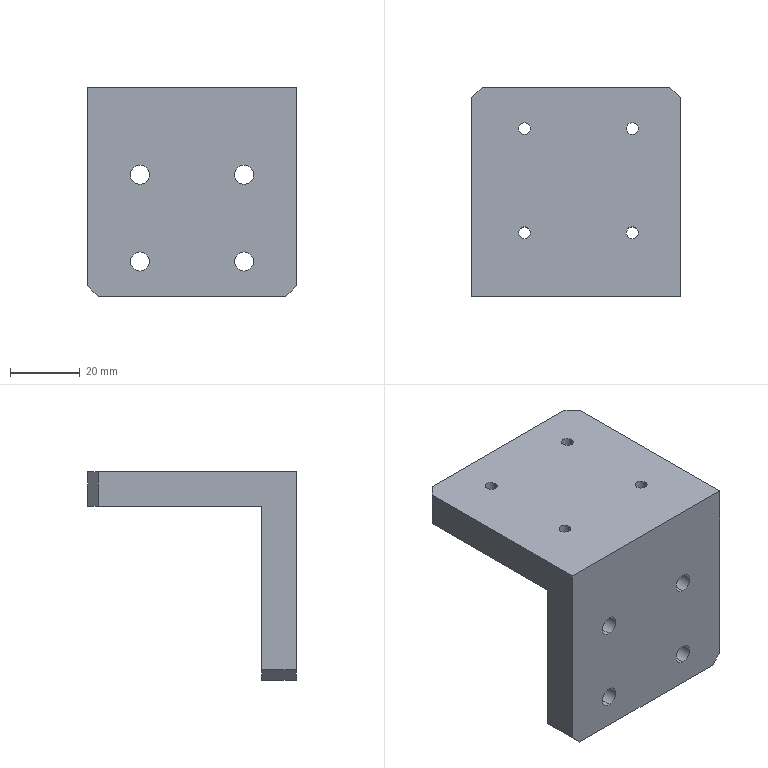Part | SolidWorks | features HoleWzd 2, Chamfer 1, Extrusion 1, ICE 1 | 1 solid | 52 faces | box 60 x 60 x 60 mm | volume 62996 mm3 | cylinder 32 | plane 20 | commonest cylinder face diameters 3.4 x8 5.5 x8 6 x8 10 x8
STEP:
#1=CARTESIAN_POINT('',(19.2,48.2,23.4));
#2=VERTEX_POINT('',#1);
#3=CARTESIAN_POINT('',(13.2,48.2,23.4));
#4=VERTEX_POINT('',#3);
#5=CARTESIAN_POINT('',(16.2,48.2,23.4));
#6=DIRECTION('',(0.,0.,-1.));
#7=DIRECTION('',(-1.,0.,0.));
#8=AXIS2_PLACEMENT_3D('',#5,#6,#7);
#9=CIRCLE('',#8,3.);
#10=EDGE_CURVE('',#2,#4,#9,.T.);
#11=ORIENTED_EDGE('',*,*,#10,.F.);
#12=CARTESIAN_POINT('',(19.2,48.2,20.));
#13=VERTEX_POINT('',#12);
#14=CARTESIAN_POINT('',(19.2,48.2,20.));
#15=DIRECTION('',(0.,0.,-1.));
#16=VECTOR('',#15,1000.);
#17=LINE('',#14,#16);
#18=EDGE_CURVE('',#2,#13,#17,.T.);
#19=ORIENTED_EDGE('',*,*,#18,.T.);
#20=CARTESIAN_POINT('',(13.2,48.2,20.));
#21=VERTEX_POINT('',#20);
#22=CARTESIAN_POINT('',(16.2,48.2,20.));
#23=DIRECTION('',(0.,0.,-1.));
#24=DIRECTION('',(-1.,0.,0.));
#25=AXIS2_PLACEMENT_3D('',#22,#23,#24);
#26=CIRCLE('',#25,3.);
#27=EDGE_CURVE('',#13,#21,#26,.T.);
#28=ORIENTED_EDGE('',*,*,#27,.T.);
#29=CARTESIAN_POINT('',(13.2,48.2,20.));
#30=DIRECTION('',(0.,0.,-1.));
#31=VECTOR('',#30,1000.);
#32=LINE('',#29,#31);
#33=EDGE_CURVE('',#4,#21,#32,.T.);
#34=ORIENTED_EDGE('',*,*,#33,.F.);
#35=EDGE_LOOP('',(#11,#19,#28,#34));
#36=FACE_OUTER_BOUND('',#35,.T.);
#37=CARTESIAN_POINT('',(16.2,48.2,20.));
#38=DIRECTION('',(0.,0.,-1.));
#39=DIRECTION('',(-1.,0.,0.));
#40=AXIS2_PLACEMENT_3D('',#37,#38,#39);
#41=CYLINDRICAL_SURFACE('',#40,3.);
#42=ADVANCED_FACE('',(#36),#41,.F.);
#43=CARTESIAN_POINT('',(17.9,48.2,30.));
#44=VERTEX_POINT('',#43);
#45=CARTESIAN_POINT('',(14.5,48.2,30.));
#46=VERTEX_POINT('',#45);
#47=CARTESIAN_POINT('',(16.2,48.2,30.));
#48=DIRECTION('',(0.,0.,-1.));
#49=DIRECTION('',(-1.,0.,0.));
#50=AXIS2_PLACEMENT_3D('',#47,#48,#49);
#51=CIRCLE('',#50,1.7);
#52=EDGE_CURVE('',#44,#46,#51,.T.);
#53=ORIENTED_EDGE('',*,*,#52,.F.);
#54=CARTESIAN_POINT('',(17.9,48.2,23.4));
#55=VERTEX_POINT('',#54);
#56=CARTESIAN_POINT('',(17.9,48.2,20.));
#57=DIRECTION('',(0.,0.,-1.));
#58=VECTOR('',#57,1000.);
#59=LINE('',#56,#58);
#60=EDGE_CURVE('',#44,#55,#59,.T.);
#61=ORIENTED_EDGE('',*,*,#60,.T.);
#62=CARTESIAN_POINT('',(14.5,48.2,23.4));
#63=VERTEX_POINT('',#62);
#64=CARTESIAN_POINT('',(16.2,48.2,23.4));
#65=DIRECTION('',(0.,0.,-1.));
#66=DIRECTION('',(-1.,0.,0.));
#67=AXIS2_PLACEMENT_3D('',#64,#65,#66);
#68=CIRCLE('',#67,1.7);
#69=EDGE_CURVE('',#55,#63,#68,.T.);
#70=ORIENTED_EDGE('',*,*,#69,.T.);
#71=CARTESIAN_POINT('',(14.5,48.2,20.));
#72=DIRECTION('',(0.,0.,-1.));
#73=VECTOR('',#72,1000.);
#74=LINE('',#71,#73);
#75=EDGE_CURVE('',#46,#63,#74,.T.);
#76=ORIENTED_EDGE('',*,*,#75,.F.);
#77=EDGE_LOOP('',(#53,#61,#70,#76));
#78=FACE_OUTER_BOUND('',#77,.T.);
#79=CARTESIAN_POINT('',(16.2,48.2,20.));
#80=DIRECTION('',(0.,0.,-1.));
#81=DIRECTION('',(-1.,0.,0.));
#82=AXIS2_PLACEMENT_3D('',#79,#80,#81);
#83=CYLINDRICAL_SURFACE('',#82,1.7);
#84=ADVANCED_FACE('',(#78),#83,.F.);
#85=CARTESIAN_POINT('',(-11.8,48.2,23.4));
#86=VERTEX_POINT('',#85);
#87=CARTESIAN_POINT('',(-17.8,48.2,23.4));
#88=VERTEX_POINT('',#87);
#89=CARTESIAN_POINT('',(-14.8,48.2,23.4));
#90=DIRECTION('',(0.,0.,-1.));
#91=DIRECTION('',(-1.,0.,0.));
#92=AXIS2_PLACEMENT_3D('',#89,#90,#91);
#93=CIRCLE('',#92,3.);
#94=EDGE_CURVE('',#86,#88,#93,.T.);
#95=ORIENTED_EDGE('',*,*,#94,.F.);
#96=CARTESIAN_POINT('',(-11.8,48.2,20.));
#97=VERTEX_POINT('',#96);
#98=CARTESIAN_POINT('',(-11.8,48.2,20.));
#99=DIRECTION('',(0.,0.,-1.));
#100=VECTOR('',#99,1000.);
#101=LINE('',#98,#100);
#102=EDGE_CURVE('',#86,#97,#101,.T.);
#103=ORIENTED_EDGE('',*,*,#102,.T.);
#104=CARTESIAN_POINT('',(-17.8,48.2,20.));
#105=VERTEX_POINT('',#104);
#106=CARTESIAN_POINT('',(-14.8,48.2,20.));
#107=DIRECTION('',(0.,0.,-1.));
#108=DIRECTION('',(-1.,0.,0.));
#109=AXIS2_PLACEMENT_3D('',#106,#107,#108);
#110=CIRCLE('',#109,3.);
#111=EDGE_CURVE('',#97,#105,#110,.T.);
#112=ORIENTED_EDGE('',*,*,#111,.T.);
#113=CARTESIAN_POINT('',(-17.8,48.2,20.));
#114=DIRECTION('',(0.,0.,-1.));
#115=VECTOR('',#114,1000.);
#116=LINE('',#113,#115);
#117=EDGE_CURVE('',#88,#105,#116,.T.);
#118=ORIENTED_EDGE('',*,*,#117,.F.);
#119=EDGE_LOOP('',(#95,#103,#112,#118));
#120=FACE_OUTER_BOUND('',#119,.T.);
#121=CARTESIAN_POINT('',(-14.8,48.2,20.));
#122=DIRECTION('',(0.,0.,-1.));
#123=DIRECTION('',(-1.,0.,0.));
#124=AXIS2_PLACEMENT_3D('',#121,#122,#123);
#125=CYLINDRICAL_SURFACE('',#124,3.);
#126=ADVANCED_FACE('',(#120),#125,.F.);
#127=CARTESIAN_POINT('',(-13.1,48.2,30.));
#128=VERTEX_POINT('',#127);
#129=CARTESIAN_POINT('',(-16.5,48.2,30.));
#130=VERTEX_POINT('',#129);
#131=CARTESIAN_POINT('',(-14.8,48.2,30.));
#132=DIRECTION('',(0.,0.,-1.));
#133=DIRECTION('',(-1.,0.,0.));
#134=AXIS2_PLACEMENT_3D('',#131,#132,#133);
#135=CIRCLE('',#134,1.7);
#136=EDGE_CURVE('',#128,#130,#135,.T.);
#137=ORIENTED_EDGE('',*,*,#136,.F.);
#138=CARTESIAN_POINT('',(-13.1,48.2,23.4));
#139=VERTEX_POINT('',#138);
#140=CARTESIAN_POINT('',(-13.1,48.2,20.));
#141=DIRECTION('',(0.,0.,-1.));
#142=VECTOR('',#141,1000.);
#143=LINE('',#140,#142);
#144=EDGE_CURVE('',#128,#139,#143,.T.);
#145=ORIENTED_EDGE('',*,*,#144,.T.);
#146=CARTESIAN_POINT('',(-16.5,48.2,23.4));
#147=VERTEX_POINT('',#146);
#148=CARTESIAN_POINT('',(-14.8,48.2,23.4));
#149=DIRECTION('',(0.,0.,-1.));
#150=DIRECTION('',(-1.,0.,0.));
#151=AXIS2_PLACEMENT_3D('',#148,#149,#150);
#152=CIRCLE('',#151,1.7);
#153=EDGE_CURVE('',#139,#147,#152,.T.);
#154=ORIENTED_EDGE('',*,*,#153,.T.);
#155=CARTESIAN_POINT('',(-16.5,48.2,20.));
#156=DIRECTION('',(0.,0.,-1.));
#157=VECTOR('',#156,1000.);
#158=LINE('',#155,#157);
#159=EDGE_CURVE('',#130,#147,#158,.T.);
#160=ORIENTED_EDGE('',*,*,#159,.F.);
#161=EDGE_LOOP('',(#137,#145,#154,#160));
#162=FACE_OUTER_BOUND('',#161,.T.);
#163=CARTESIAN_POINT('',(-14.8,48.2,20.));
#164=DIRECTION('',(0.,0.,-1.));
#165=DIRECTION('',(-1.,0.,0.));
#166=AXIS2_PLACEMENT_3D('',#163,#164,#165);
#167=CYLINDRICAL_SURFACE('',#166,1.7);
#168=ADVANCED_FACE('',(#162),#167,.F.);
#169=CARTESIAN_POINT('',(19.2,18.2,23.4));
#170=VERTEX_POINT('',#169);
#171=CARTESIAN_POINT('',(13.2,18.2,23.4));
#172=VERTEX_POINT('',#171);
#173=CARTESIAN_POINT('',(16.2,18.2,23.4));
#174=DIRECTION('',(0.,0.,-1.));
#175=DIRECTION('',(-1.,0.,0.));
#176=AXIS2_PLACEMENT_3D('',#173,#174,#175);
#177=CIRCLE('',#176,3.);
#178=EDGE_CURVE('',#170,#172,#177,.T.);
#179=ORIENTED_EDGE('',*,*,#178,.F.);
#180=CARTESIAN_POINT('',(19.2,18.2,20.));
#181=VERTEX_POINT('',#180);
#182=CARTESIAN_POINT('',(19.2,18.2,20.));
#183=DIRECTION('',(0.,0.,-1.));
#184=VECTOR('',#183,1000.);
#185=LINE('',#182,#184);
#186=EDGE_CURVE('',#170,#181,#185,.T.);
#187=ORIENTED_EDGE('',*,*,#186,.T.);
#188=CARTESIAN_POINT('',(13.2,18.2,20.));
#189=VERTEX_POINT('',#188);
#190=CARTESIAN_POINT('',(16.2,18.2,20.));
#191=DIRECTION('',(0.,0.,-1.));
#192=DIRECTION('',(-1.,0.,0.));
#193=AXIS2_PLACEMENT_3D('',#190,#191,#192);
#194=CIRCLE('',#193,3.);
#195=EDGE_CURVE('',#181,#189,#194,.T.);
#196=ORIENTED_EDGE('',*,*,#195,.T.);
#197=CARTESIAN_POINT('',(13.2,18.2,20.));
#198=DIRECTION('',(0.,0.,-1.));
#199=VECTOR('',#198,1000.);
#200=LINE('',#197,#199);
#201=EDGE_CURVE('',#172,#189,#200,.T.);
#202=ORIENTED_EDGE('',*,*,#201,.F.);
#203=EDGE_LOOP('',(#179,#187,#196,#202));
#204=FACE_OUTER_BOUND('',#203,.T.);
#205=CARTESIAN_POINT('',(16.2,18.2,20.));
#206=DIRECTION('',(0.,0.,-1.));
#207=DIRECTION('',(-1.,0.,0.));
#208=AXIS2_PLACEMENT_3D('',#205,#206,#207);
#209=CYLINDRICAL_SURFACE('',#208,3.);
#210=ADVANCED_FACE('',(#204),#209,.F.);
#211=CARTESIAN_POINT('',(17.9,18.2,30.));
#212=VERTEX_POINT('',#211);
#213=CARTESIAN_POINT('',(14.5,18.2,30.));
#214=VERTEX_POINT('',#213);
#215=CARTESIAN_POINT('',(16.2,18.2,30.));
#216=DIRECTION('',(0.,0.,-1.));
#217=DIRECTION('',(-1.,0.,0.));
#218=AXIS2_PLACEMENT_3D('',#215,#216,#217);
#219=CIRCLE('',#218,1.7);
#220=EDGE_CURVE('',#212,#214,#219,.T.);
#221=ORIENTED_EDGE('',*,*,#220,.F.);
#222=CARTESIAN_POINT('',(17.9,18.2,23.4));
#223=VERTEX_POINT('',#222);
#224=CARTESIAN_POINT('',(17.9,18.2,20.));
#225=DIRECTION('',(0.,0.,-1.));
#226=VECTOR('',#225,1000.);
#227=LINE('',#224,#226);
#228=EDGE_CURVE('',#212,#223,#227,.T.);
#229=ORIENTED_EDGE('',*,*,#228,.T.);
#230=CARTESIAN_POINT('',(14.5,18.2,23.4));
#231=VERTEX_POINT('',#230);
#232=CARTESIAN_POINT('',(16.2,18.2,23.4));
#233=DIRECTION('',(0.,0.,-1.));
#234=DIRECTION('',(-1.,0.,0.));
#235=AXIS2_PLACEMENT_3D('',#232,#233,#234);
#236=CIRCLE('',#235,1.7);
#237=EDGE_CURVE('',#223,#231,#236,.T.);
#238=ORIENTED_EDGE('',*,*,#237,.T.);
#239=CARTESIAN_POINT('',(14.5,18.2,20.));
#240=DIRECTION('',(0.,0.,-1.));
#241=VECTOR('',#240,1000.);
#242=LINE('',#239,#241);
#243=EDGE_CURVE('',#214,#231,#242,.T.);
#244=ORIENTED_EDGE('',*,*,#243,.F.);
#245=EDGE_LOOP('',(#221,#229,#238,#244));
#246=FACE_OUTER_BOUND('',#245,.T.);
#247=CARTESIAN_POINT('',(16.2,18.2,20.));
#248=DIRECTION('',(0.,0.,-1.));
#249=DIRECTION('',(-1.,0.,0.));
#250=AXIS2_PLACEMENT_3D('',#247,#248,#249);
#251=CYLINDRICAL_SURFACE('',#250,1.7);
#252=ADVANCED_FACE('',(#246),#251,.F.);
#253=CARTESIAN_POINT('',(-11.8,18.2,23.4));
#254=VERTEX_POINT('',#253);
#255=CARTESIAN_POINT('',(-17.8,18.2,23.4));
#256=VERTEX_POINT('',#255);
#257=CARTESIAN_POINT('',(-14.8,18.2,23.4));
#258=DIRECTION('',(0.,0.,-1.));
#259=DIRECTION('',(-1.,0.,0.));
#260=AXIS2_PLACEMENT_3D('',#257,#258,#259);
#261=CIRCLE('',#260,3.);
#262=EDGE_CURVE('',#254,#256,#261,.T.);
#263=ORIENTED_EDGE('',*,*,#262,.F.);
#264=CARTESIAN_POINT('',(-11.8,18.2,20.));
#265=VERTEX_POINT('',#264);
#266=CARTESIAN_POINT('',(-11.8,18.2,20.));
#267=DIRECTION('',(0.,0.,-1.));
#268=VECTOR('',#267,1000.);
#269=LINE('',#266,#268);
#270=EDGE_CURVE('',#254,#265,#269,.T.);
#271=ORIENTED_EDGE('',*,*,#270,.T.);
#272=CARTESIAN_POINT('',(-17.8,18.2,20.));
#273=VERTEX_POINT('',#272);
#274=CARTESIAN_POINT('',(-14.8,18.2,20.));
#275=DIRECTION('',(0.,0.,-1.));
#276=DIRECTION('',(-1.,0.,0.));
#277=AXIS2_PLACEMENT_3D('',#274,#275,#276);
#278=CIRCLE('',#277,3.);
#279=EDGE_CURVE('',#265,#273,#278,.T.);
#280=ORIENTED_EDGE('',*,*,#279,.T.);
#281=CARTESIAN_POINT('',(-17.8,18.2,20.));
#282=DIRECTION('',(0.,0.,-1.));
#283=VECTOR('',#282,1000.);
#284=LINE('',#281,#283);
#285=EDGE_CURVE('',#256,#273,#284,.T.);
#286=ORIENTED_EDGE('',*,*,#285,.F.);
#287=EDGE_LOOP('',(#263,#271,#280,#286));
#288=FACE_OUTER_BOUND('',#287,.T.);
#289=CARTESIAN_POINT('',(-14.8,18.2,20.));
#290=DIRECTION('',(0.,0.,-1.));
#291=DIRECTION('',(-1.,0.,0.));
#292=AXIS2_PLACEMENT_3D('',#289,#290,#291);
#293=CYLINDRICAL_SURFACE('',#292,3.);
#294=ADVANCED_FACE('',(#288),#293,.F.);
#295=CARTESIAN_POINT('',(-13.1,18.2,30.));
#296=VERTEX_POINT('',#295);
#297=CARTESIAN_POINT('',(-16.5,18.2,30.));
#298=VERTEX_POINT('',#297);
#299=CARTESIAN_POINT('',(-14.8,18.2,30.));
#300=DIRECTION('',(0.,0.,-1.));
#301=DIRECTION('',(-1.,0.,0.));
#302=AXIS2_PLACEMENT_3D('',#299,#300,#301);
#303=CIRCLE('',#302,1.7);
#304=EDGE_CURVE('',#296,#298,#303,.T.);
#305=ORIENTED_EDGE('',*,*,#304,.F.);
#306=CARTESIAN_POINT('',(-13.1,18.2,23.4));
#307=VERTEX_POINT('',#306);
#308=CARTESIAN_POINT('',(-13.1,18.2,20.));
#309=DIRECTION('',(0.,0.,-1.));
#310=VECTOR('',#309,1000.);
#311=LINE('',#308,#310);
#312=EDGE_CURVE('',#296,#307,#311,.T.);
#313=ORIENTED_EDGE('',*,*,#312,.T.);
#314=CARTESIAN_POINT('',(-16.5,18.2,23.4));
#315=VERTEX_POINT('',#314);
#316=CARTESIAN_POINT('',(-14.8,18.2,23.4));
#317=DIRECTION('',(0.,0.,-1.));
#318=DIRECTION('',(-1.,0.,0.));
#319=AXIS2_PLACEMENT_3D('',#316,#317,#318);
#320=CIRCLE('',#319,1.7);
#321=EDGE_CURVE('',#307,#315,#320,.T.);
#322=ORIENTED_EDGE('',*,*,#321,.T.);
#323=CARTESIAN_POINT('',(-16.5,18.2,20.));
#324=DIRECTION('',(0.,0.,-1.));
#325=VECTOR('',#324,1000.);
#326=LINE('',#323,#325);
#327=EDGE_CURVE('',#298,#315,#326,.T.);
#328=ORIENTED_EDGE('',*,*,#327,.F.);
#329=EDGE_LOOP('',(#305,#313,#322,#328));
#330=FACE_OUTER_BOUND('',#329,.T.);
#331=CARTESIAN_POINT('',(-14.8,18.2,20.));
#332=DIRECTION('',(0.,0.,-1.));
#333=DIRECTION('',(-1.,0.,0.));
#334=AXIS2_PLACEMENT_3D('',#331,#332,#333);
#335=CYLINDRICAL_SURFACE('',#334,1.7);
#336=ADVANCED_FACE('',(#330),#335,.F.);
#337=CARTESIAN_POINT('',(-15.,4.3,-25.));
#338=VERTEX_POINT('',#337);
#339=CARTESIAN_POINT('',(-15.,4.3,-15.));
#340=VERTEX_POINT('',#339);
#341=CARTESIAN_POINT('',(-15.,4.3,-20.));
#342=DIRECTION('',(0.,1.,0.));
#343=DIRECTION('',(0.,0.,1.));
#344=AXIS2_PLACEMENT_3D('',#341,#342,#343);
#345=CIRCLE('',#344,5.);
#346=EDGE_CURVE('',#338,#340,#345,.T.);
#347=ORIENTED_EDGE('',*,*,#346,.F.);
#348=CARTESIAN_POINT('',(-15.,10.,-25.));
#349=VERTEX_POINT('',#348);
#350=CARTESIAN_POINT('',(-15.,10.,-25.));
#351=DIRECTION('',(0.,1.,0.));
#352=VECTOR('',#351,1000.);
#353=LINE('',#350,#352);
#354=EDGE_CURVE('',#338,#349,#353,.T.);
#355=ORIENTED_EDGE('',*,*,#354,.T.);
#356=CARTESIAN_POINT('',(-15.,10.,-15.));
#357=VERTEX_POINT('',#356);
#358=CARTESIAN_POINT('',(-15.,10.,-20.));
#359=DIRECTION('',(0.,1.,0.));
#360=DIRECTION('',(0.,0.,1.));
#361=AXIS2_PLACEMENT_3D('',#358,#359,#360);
#362=CIRCLE('',#361,5.);
#363=EDGE_CURVE('',#349,#357,#362,.T.);
#364=ORIENTED_EDGE('',*,*,#363,.T.);
#365=CARTESIAN_POINT('',(-15.,10.,-15.));
#366=DIRECTION('',(0.,1.,0.));
#367=VECTOR('',#366,1000.);
#368=LINE('',#365,#367);
#369=EDGE_CURVE('',#340,#357,#368,.T.);
#370=ORIENTED_EDGE('',*,*,#369,.F.);
#371=EDGE_LOOP('',(#347,#355,#364,#370));
#372=FACE_OUTER_BOUND('',#371,.T.);
#373=CARTESIAN_POINT('',(-15.,10.,-20.));
#374=DIRECTION('',(0.,1.,0.));
#375=DIRECTION('',(0.,0.,1.));
#376=AXIS2_PLACEMENT_3D('',#373,#374,#375);
#377=CYLINDRICAL_SURFACE('',#376,5.);
#378=ADVANCED_FACE('',(#372),#377,.F.);
#379=CARTESIAN_POINT('',(-15.,0.,-22.75));
#380=VERTEX_POINT('',#379);
#381=CARTESIAN_POINT('',(-15.,0.,-17.25));
#382=VERTEX_POINT('',#381);
#383=CARTESIAN_POINT('',(-15.,0.,-20.));
#384=DIRECTION('',(0.,1.,0.));
#385=DIRECTION('',(0.,0.,1.));
#386=AXIS2_PLACEMENT_3D('',#383,#384,#385);
#387=CIRCLE('',#386,2.75);
#388=EDGE_CURVE('',#380,#382,#387,.T.);
#389=ORIENTED_EDGE('',*,*,#388,.F.);
#390=CARTESIAN_POINT('',(-15.,4.3,-22.75));
#391=VERTEX_POINT('',#390);
#392=CARTESIAN_POINT('',(-15.,10.,-22.75));
#393=DIRECTION('',(0.,1.,0.));
#394=VECTOR('',#393,1000.);
#395=LINE('',#392,#394);
#396=EDGE_CURVE('',#380,#391,#395,.T.);
#397=ORIENTED_EDGE('',*,*,#396,.T.);
#398=CARTESIAN_POINT('',(-15.,4.3,-17.25));
#399=VERTEX_POINT('',#398);
#400=CARTESIAN_POINT('',(-15.,4.3,-20.));
#401=DIRECTION('',(0.,1.,0.));
#402=DIRECTION('',(0.,0.,1.));
#403=AXIS2_PLACEMENT_3D('',#400,#401,#402);
#404=CIRCLE('',#403,2.75);
#405=EDGE_CURVE('',#391,#399,#404,.T.);
#406=ORIENTED_EDGE('',*,*,#405,.T.);
#407=CARTESIAN_POINT('',(-15.,10.,-17.25));
#408=DIRECTION('',(0.,1.,0.));
#409=VECTOR('',#408,1000.);
#410=LINE('',#407,#409);
#411=EDGE_CURVE('',#382,#399,#410,.T.);
#412=ORIENTED_EDGE('',*,*,#411,.F.);
#413=EDGE_LOOP('',(#389,#397,#406,#412));
#414=FACE_OUTER_BOUND('',#413,.T.);
#415=CARTESIAN_POINT('',(-15.,10.,-20.));
#416=DIRECTION('',(0.,1.,0.));
#417=DIRECTION('',(0.,0.,1.));
#418=AXIS2_PLACEMENT_3D('',#415,#416,#417);
#419=CYLINDRICAL_SURFACE('',#418,2.75);
#420=ADVANCED_FACE('',(#414),#419,.F.);
#421=CARTESIAN_POINT('',(15.,4.3,-25.));
#422=VERTEX_POINT('',#421);
#423=CARTESIAN_POINT('',(15.,4.3,-15.));
#424=VERTEX_POINT('',#423);
#425=CARTESIAN_POINT('',(15.,4.3,-20.));
#426=DIRECTION('',(0.,1.,0.));
#427=DIRECTION('',(0.,0.,1.));
#428=AXIS2_PLACEMENT_3D('',#425,#426,#427);
#429=CIRCLE('',#428,5.);
#430=EDGE_CURVE('',#422,#424,#429,.T.);
#431=ORIENTED_EDGE('',*,*,#430,.F.);
#432=CARTESIAN_POINT('',(15.,10.,-25.));
#433=VERTEX_POINT('',#432);
#434=CARTESIAN_POINT('',(15.,10.,-25.));
#435=DIRECTION('',(0.,1.,0.));
#436=VECTOR('',#435,1000.);
#437=LINE('',#434,#436);
#438=EDGE_CURVE('',#422,#433,#437,.T.);
#439=ORIENTED_EDGE('',*,*,#438,.T.);
#440=CARTESIAN_POINT('',(15.,10.,-15.));
#441=VERTEX_POINT('',#440);
#442=CARTESIAN_POINT('',(15.,10.,-20.));
#443=DIRECTION('',(0.,1.,0.));
#444=DIRECTION('',(0.,0.,1.));
#445=AXIS2_PLACEMENT_3D('',#442,#443,#444);
#446=CIRCLE('',#445,5.);
#447=EDGE_CURVE('',#433,#441,#446,.T.);
#448=ORIENTED_EDGE('',*,*,#447,.T.);
#449=CARTESIAN_POINT('',(15.,10.,-15.));
#450=DIRECTION('',(0.,1.,0.));
#451=VECTOR('',#450,1000.);
#452=LINE('',#449,#451);
#453=EDGE_CURVE('',#424,#441,#452,.T.);
#454=ORIENTED_EDGE('',*,*,#453,.F.);
#455=EDGE_LOOP('',(#431,#439,#448,#454));
#456=FACE_OUTER_BOUND('',#455,.T.);
#457=CARTESIAN_POINT('',(15.,10.,-20.));
#458=DIRECTION('',(0.,1.,0.));
#459=DIRECTION('',(0.,0.,1.));
#460=AXIS2_PLACEMENT_3D('',#457,#458,#459);
#461=CYLINDRICAL_SURFACE('',#460,5.);
#462=ADVANCED_FACE('',(#456),#461,.F.);
#463=CARTESIAN_POINT('',(15.,0.,-22.75));
#464=VERTEX_POINT('',#463);
#465=CARTESIAN_POINT('',(15.,0.,-17.25));
#466=VERTEX_POINT('',#465);
#467=CARTESIAN_POINT('',(15.,0.,-20.));
#468=DIRECTION('',(0.,1.,0.));
#469=DIRECTION('',(0.,0.,1.));
#470=AXIS2_PLACEMENT_3D('',#467,#468,#469);
#471=CIRCLE('',#470,2.75);
#472=EDGE_CURVE('',#464,#466,#471,.T.);
#473=ORIENTED_EDGE('',*,*,#472,.F.);
#474=CARTESIAN_POINT('',(15.,4.3,-22.75));
#475=VERTEX_POINT('',#474);
#476=CARTESIAN_POINT('',(15.,10.,-22.75));
#477=DIRECTION('',(0.,1.,0.));
#478=VECTOR('',#477,1000.);
#479=LINE('',#476,#478);
#480=EDGE_CURVE('',#464,#475,#479,.T.);
#481=ORIENTED_EDGE('',*,*,#480,.T.);
#482=CARTESIAN_POINT('',(15.,4.3,-17.25));
#483=VERTEX_POINT('',#482);
#484=CARTESIAN_POINT('',(15.,4.3,-20.));
#485=DIRECTION('',(0.,1.,0.));
#486=DIRECTION('',(0.,0.,1.));
#487=AXIS2_PLACEMENT_3D('',#484,#485,#486);
#488=CIRCLE('',#487,2.75);
#489=EDGE_CURVE('',#475,#483,#488,.T.);
#490=ORIENTED_EDGE('',*,*,#489,.T.);
#491=CARTESIAN_POINT('',(15.,10.,-17.25));
#492=DIRECTION('',(0.,1.,0.));
#493=VECTOR('',#492,1000.);
#494=LINE('',#491,#493);
#495=EDGE_CURVE('',#466,#483,#494,.T.);
#496=ORIENTED_EDGE('',*,*,#495,.F.);
#497=EDGE_LOOP('',(#473,#481,#490,#496));
#498=FACE_OUTER_BOUND('',#497,.T.);
#499=CARTESIAN_POINT('',(15.,10.,-20.));
#500=DIRECTION('',(0.,1.,0.));
#501=DIRECTION('',(0.,0.,1.));
#502=AXIS2_PLACEMENT_3D('',#499,#500,#501);
#503=CYLINDRICAL_SURFACE('',#502,2.75);
#504=ADVANCED_FACE('',(#498),#503,.F.);
#505=CARTESIAN_POINT('',(-15.,4.3,0.));
#506=VERTEX_POINT('',#505);
#507=CARTESIAN_POINT('',(-15.,4.3,10.));
#508=VERTEX_POINT('',#507);
#509=CARTESIAN_POINT('',(-15.,4.3,5.));
#510=DIRECTION('',(0.,1.,0.));
#511=DIRECTION('',(0.,0.,1.));
#512=AXIS2_PLACEMENT_3D('',#509,#510,#511);
#513=CIRCLE('',#512,5.);
#514=EDGE_CURVE('',#506,#508,#513,.T.);
#515=ORIENTED_EDGE('',*,*,#514,.F.);
#516=CARTESIAN_POINT('',(-15.,10.,0.));
#517=VERTEX_POINT('',#516);
#518=CARTESIAN_POINT('',(-15.,10.,0.));
#519=DIRECTION('',(0.,1.,0.));
#520=VECTOR('',#519,1000.);
#521=LINE('',#518,#520);
#522=EDGE_CURVE('',#506,#517,#521,.T.);
#523=ORIENTED_EDGE('',*,*,#522,.T.);
#524=CARTESIAN_POINT('',(-15.,10.,10.));
#525=VERTEX_POINT('',#524);
#526=CARTESIAN_POINT('',(-15.,10.,5.));
#527=DIRECTION('',(0.,1.,0.));
#528=DIRECTION('',(0.,0.,1.));
#529=AXIS2_PLACEMENT_3D('',#526,#527,#528);
#530=CIRCLE('',#529,5.);
#531=EDGE_CURVE('',#517,#525,#530,.T.);
#532=ORIENTED_EDGE('',*,*,#531,.T.);
#533=CARTESIAN_POINT('',(-15.,10.,10.));
#534=DIRECTION('',(0.,1.,0.));
#535=VECTOR('',#534,1000.);
#536=LINE('',#533,#535);
#537=EDGE_CURVE('',#508,#525,#536,.T.);
#538=ORIENTED_EDGE('',*,*,#537,.F.);
#539=EDGE_LOOP('',(#515,#523,#532,#538));
#540=FACE_OUTER_BOUND('',#539,.T.);
#541=CARTESIAN_POINT('',(-15.,10.,5.));
#542=DIRECTION('',(0.,1.,0.));
#543=DIRECTION('',(0.,0.,1.));
#544=AXIS2_PLACEMENT_3D('',#541,#542,#543);
#545=CYLINDRICAL_SURFACE('',#544,5.);
#546=ADVANCED_FACE('',(#540),#545,.F.);
#547=CARTESIAN_POINT('',(-15.,0.,2.25));
#548=VERTEX_POINT('',#547);
#549=CARTESIAN_POINT('',(-15.,0.,7.75));
#550=VERTEX_POINT('',#549);
#551=CARTESIAN_POINT('',(-15.,0.,5.));
#552=DIRECTION('',(0.,1.,0.));
#553=DIRECTION('',(0.,0.,1.));
#554=AXIS2_PLACEMENT_3D('',#551,#552,#553);
#555=CIRCLE('',#554,2.75);
#556=EDGE_CURVE('',#548,#550,#555,.T.);
#557=ORIENTED_EDGE('',*,*,#556,.F.);
#558=CARTESIAN_POINT('',(-15.,4.3,2.25));
#559=VERTEX_POINT('',#558);
#560=CARTESIAN_POINT('',(-15.,10.,2.25));
#561=DIRECTION('',(0.,1.,0.));
#562=VECTOR('',#561,1000.);
#563=LINE('',#560,#562);
#564=EDGE_CURVE('',#548,#559,#563,.T.);
#565=ORIENTED_EDGE('',*,*,#564,.T.);
#566=CARTESIAN_POINT('',(-15.,4.3,7.75));
#567=VERTEX_POINT('',#566);
#568=CARTESIAN_POINT('',(-15.,4.3,5.));
#569=DIRECTION('',(0.,1.,0.));
#570=DIRECTION('',(0.,0.,1.));
#571=AXIS2_PLACEMENT_3D('',#568,#569,#570);
#572=CIRCLE('',#571,2.75);
#573=EDGE_CURVE('',#559,#567,#572,.T.);
#574=ORIENTED_EDGE('',*,*,#573,.T.);
#575=CARTESIAN_POINT('',(-15.,10.,7.75));
#576=DIRECTION('',(0.,1.,0.));
#577=VECTOR('',#576,1000.);
#578=LINE('',#575,#577);
#579=EDGE_CURVE('',#550,#567,#578,.T.);
#580=ORIENTED_EDGE('',*,*,#579,.F.);
#581=EDGE_LOOP('',(#557,#565,#574,#580));
#582=FACE_OUTER_BOUND('',#581,.T.);
#583=CARTESIAN_POINT('',(-15.,10.,5.));
#584=DIRECTION('',(0.,1.,0.));
#585=DIRECTION('',(0.,0.,1.));
#586=AXIS2_PLACEMENT_3D('',#583,#584,#585);
#587=CYLINDRICAL_SURFACE('',#586,2.75);
#588=ADVANCED_FACE('',(#582),#587,.F.);
#589=CARTESIAN_POINT('',(15.,4.3,0.));
#590=VERTEX_POINT('',#589);
#591=CARTESIAN_POINT('',(15.,4.3,10.));
#592=VERTEX_POINT('',#591);
#593=CARTESIAN_POINT('',(15.,4.3,5.));
#594=DIRECTION('',(0.,1.,0.));
#595=DIRECTION('',(0.,0.,1.));
#596=AXIS2_PLACEMENT_3D('',#593,#594,#595);
#597=CIRCLE('',#596,5.);
#598=EDGE_CURVE('',#590,#592,#597,.T.);
#599=ORIENTED_EDGE('',*,*,#598,.F.);
#600=CARTESIAN_POINT('',(15.,10.,0.));
#601=VERTEX_POINT('',#600);
#602=CARTESIAN_POINT('',(15.,10.,0.));
#603=DIRECTION('',(0.,1.,0.));
#604=VECTOR('',#603,1000.);
#605=LINE('',#602,#604);
#606=EDGE_CURVE('',#590,#601,#605,.T.);
#607=ORIENTED_EDGE('',*,*,#606,.T.);
#608=CARTESIAN_POINT('',(15.,10.,10.));
#609=VERTEX_POINT('',#608);
#610=CARTESIAN_POINT('',(15.,10.,5.));
#611=DIRECTION('',(0.,1.,0.));
#612=DIRECTION('',(0.,0.,1.));
#613=AXIS2_PLACEMENT_3D('',#610,#611,#612);
#614=CIRCLE('',#613,5.);
#615=EDGE_CURVE('',#601,#609,#614,.T.);
#616=ORIENTED_EDGE('',*,*,#615,.T.);
#617=CARTESIAN_POINT('',(15.,10.,10.));
#618=DIRECTION('',(0.,1.,0.));
#619=VECTOR('',#618,1000.);
#620=LINE('',#617,#619);
#621=EDGE_CURVE('',#592,#609,#620,.T.);
#622=ORIENTED_EDGE('',*,*,#621,.F.);
#623=EDGE_LOOP('',(#599,#607,#616,#622));
#624=FACE_OUTER_BOUND('',#623,.T.);
#625=CARTESIAN_POINT('',(15.,10.,5.));
#626=DIRECTION('',(0.,1.,0.));
#627=DIRECTION('',(0.,0.,1.));
#628=AXIS2_PLACEMENT_3D('',#625,#626,#627);
#629=CYLINDRICAL_SURFACE('',#628,5.);
#630=ADVANCED_FACE('',(#624),#629,.F.);
#631=CARTESIAN_POINT('',(15.,0.,2.25));
#632=VERTEX_POINT('',#631);
#633=CARTESIAN_POINT('',(15.,0.,7.75));
#634=VERTEX_POINT('',#633);
#635=CARTESIAN_POINT('',(15.,0.,5.));
#636=DIRECTION('',(0.,1.,0.));
#637=DIRECTION('',(0.,0.,1.));
#638=AXIS2_PLACEMENT_3D('',#635,#636,#637);
#639=CIRCLE('',#638,2.75);
#640=EDGE_CURVE('',#632,#634,#639,.T.);
#641=ORIENTED_EDGE('',*,*,#640,.F.);
#642=CARTESIAN_POINT('',(15.,4.3,2.25));
#643=VERTEX_POINT('',#642);
#644=CARTESIAN_POINT('',(15.,10.,2.25));
#645=DIRECTION('',(0.,1.,0.));
#646=VECTOR('',#645,1000.);
#647=LINE('',#644,#646);
#648=EDGE_CURVE('',#632,#643,#647,.T.);
#649=ORIENTED_EDGE('',*,*,#648,.T.);
#650=CARTESIAN_POINT('',(15.,4.3,7.75));
#651=VERTEX_POINT('',#650);
#652=CARTESIAN_POINT('',(15.,4.3,5.));
#653=DIRECTION('',(0.,1.,0.));
#654=DIRECTION('',(0.,0.,1.));
#655=AXIS2_PLACEMENT_3D('',#652,#653,#654);
#656=CIRCLE('',#655,2.75);
#657=EDGE_CURVE('',#643,#651,#656,.T.);
#658=ORIENTED_EDGE('',*,*,#657,.T.);
#659=CARTESIAN_POINT('',(15.,10.,7.75));
#660=DIRECTION('',(0.,1.,0.));
#661=VECTOR('',#660,1000.);
#662=LINE('',#659,#661);
#663=EDGE_CURVE('',#634,#651,#662,.T.);
#664=ORIENTED_EDGE('',*,*,#663,.F.);
#665=EDGE_LOOP('',(#641,#649,#658,#664));
#666=FACE_OUTER_BOUND('',#665,.T.);
#667=CARTESIAN_POINT('',(15.,10.,5.));
#668=DIRECTION('',(0.,1.,0.));
#669=DIRECTION('',(0.,0.,1.));
#670=AXIS2_PLACEMENT_3D('',#667,#668,#669);
#671=CYLINDRICAL_SURFACE('',#670,2.75);
#672=ADVANCED_FACE('',(#666),#671,.F.);
#673=CARTESIAN_POINT('',(30.,57.,20.));
#674=VERTEX_POINT('',#673);
#675=CARTESIAN_POINT('',(30.,10.,20.));
#676=VERTEX_POINT('',#675);
#677=CARTESIAN_POINT('',(30.,60.,20.));
#678=DIRECTION('',(0.,-1.,0.));
#679=VECTOR('',#678,1000.);
#680=LINE('',#677,#679);
#681=EDGE_CURVE('',#674,#676,#680,.T.);
#682=ORIENTED_EDGE('',*,*,#681,.F.);
#683=CARTESIAN_POINT('',(30.,57.,30.));
#684=VERTEX_POINT('',#683);
#685=CARTESIAN_POINT('',(30.,57.,-30.));
#686=DIRECTION('',(0.,0.,1.));
#687=VECTOR('',#686,1000.);
#688=LINE('',#685,#687);
#689=EDGE_CURVE('',#674,#684,#688,.T.);
#690=ORIENTED_EDGE('',*,*,#689,.T.);
#691=CARTESIAN_POINT('',(30.,0.,30.));
#692=VERTEX_POINT('',#691);
#693=CARTESIAN_POINT('',(30.,10.,30.));
#694=DIRECTION('',(0.,-1.,0.));
#695=VECTOR('',#694,1000.);
#696=LINE('',#693,#695);
#697=EDGE_CURVE('',#684,#692,#696,.T.);
#698=ORIENTED_EDGE('',*,*,#697,.T.);
#699=CARTESIAN_POINT('',(30.,0.,-27.));
#700=VERTEX_POINT('',#699);
#701=CARTESIAN_POINT('',(30.,0.,-30.));
#702=DIRECTION('',(0.,0.,-1.));
#703=VECTOR('',#702,1000.);
#704=LINE('',#701,#703);
#705=EDGE_CURVE('',#692,#700,#704,.T.);
#706=ORIENTED_EDGE('',*,*,#705,.T.);
#707=CARTESIAN_POINT('',(30.,10.,-27.));
#708=VERTEX_POINT('',#707);
#709=CARTESIAN_POINT('',(30.,10.,-27.));
#710=DIRECTION('',(0.,1.,0.));
#711=VECTOR('',#710,1000.);
#712=LINE('',#709,#711);
#713=EDGE_CURVE('',#700,#708,#712,.T.);
#714=ORIENTED_EDGE('',*,*,#713,.T.);
#715=CARTESIAN_POINT('',(30.,10.,-30.));
#716=DIRECTION('',(0.,0.,-1.));
#717=VECTOR('',#716,1000.);
#718=LINE('',#715,#717);
#719=EDGE_CURVE('',#676,#708,#718,.T.);
#720=ORIENTED_EDGE('',*,*,#719,.F.);
#721=EDGE_LOOP('',(#682,#690,#698,#706,#714,#720));
#722=FACE_OUTER_BOUND('',#721,.T.);
#723=CARTESIAN_POINT('',(30.,10.,-30.));
#724=DIRECTION('',(-1.,0.,0.));
#725=DIRECTION('',(0.,0.,1.));
#726=AXIS2_PLACEMENT_3D('',#723,#724,#725);
#727=PLANE('',#726);
#728=ADVANCED_FACE('',(#722),#727,.F.);
#729=CARTESIAN_POINT('',(27.,10.,-30.));
#730=VERTEX_POINT('',#729);
#731=CARTESIAN_POINT('',(-27.,10.,-30.));
#732=VERTEX_POINT('',#731);
#733=CARTESIAN_POINT('',(-30.,10.,-30.));
#734=DIRECTION('',(-1.,0.,0.));
#735=VECTOR('',#734,1000.);
#736=LINE('',#733,#735);
#737=EDGE_CURVE('',#730,#732,#736,.T.);
#738=ORIENTED_EDGE('',*,*,#737,.F.);
#739=CARTESIAN_POINT('',(27.,0.,-30.));
#740=VERTEX_POINT('',#739);
#741=CARTESIAN_POINT('',(27.,10.,-30.));
#742=DIRECTION('',(0.,-1.,0.));
#743=VECTOR('',#742,1000.);
#744=LINE('',#741,#743);
#745=EDGE_CURVE('',#730,#740,#744,.T.);
#746=ORIENTED_EDGE('',*,*,#745,.T.);
#747=CARTESIAN_POINT('',(-27.,0.,-30.));
#748=VERTEX_POINT('',#747);
#749=CARTESIAN_POINT('',(-30.,0.,-30.));
#750=DIRECTION('',(-1.,0.,0.));
#751=VECTOR('',#750,1000.);
#752=LINE('',#749,#751);
#753=EDGE_CURVE('',#740,#748,#752,.T.);
#754=ORIENTED_EDGE('',*,*,#753,.T.);
#755=CARTESIAN_POINT('',(-27.,10.,-30.));
#756=DIRECTION('',(0.,1.,0.));
#757=VECTOR('',#756,1000.);
#758=LINE('',#755,#757);
#759=EDGE_CURVE('',#748,#732,#758,.T.);
#760=ORIENTED_EDGE('',*,*,#759,.T.);
#761=EDGE_LOOP('',(#738,#746,#754,#760));
#762=FACE_OUTER_BOUND('',#761,.T.);
#763=CARTESIAN_POINT('',(-30.,10.,-30.));
#764=DIRECTION('',(0.,0.,1.));
#765=DIRECTION('',(1.,0.,0.));
#766=AXIS2_PLACEMENT_3D('',#763,#764,#765);
#767=PLANE('',#766);
#768=ADVANCED_FACE('',(#762),#767,.F.);
#769=CARTESIAN_POINT('',(-30.,57.,30.));
#770=VERTEX_POINT('',#769);
#771=CARTESIAN_POINT('',(-30.,0.,30.));
#772=VERTEX_POINT('',#771);
#773=CARTESIAN_POINT('',(-30.,10.,30.));
#774=DIRECTION('',(0.,-1.,0.));
#775=VECTOR('',#774,1000.);
#776=LINE('',#773,#775);
#777=EDGE_CURVE('',#770,#772,#776,.T.);
#778=ORIENTED_EDGE('',*,*,#777,.F.);
#779=CARTESIAN_POINT('',(-30.,57.,20.));
#780=VERTEX_POINT('',#779);
#781=CARTESIAN_POINT('',(-30.,57.,-30.));
#782=DIRECTION('',(0.,0.,-1.));
#783=VECTOR('',#782,1000.);
#784=LINE('',#781,#783);
#785=EDGE_CURVE('',#770,#780,#784,.T.);
#786=ORIENTED_EDGE('',*,*,#785,.T.);
#787=CARTESIAN_POINT('',(-30.,10.,20.));
#788=VERTEX_POINT('',#787);
#789=CARTESIAN_POINT('',(-30.,60.,20.));
#790=DIRECTION('',(0.,-1.,0.));
#791=VECTOR('',#790,1000.);
#792=LINE('',#789,#791);
#793=EDGE_CURVE('',#780,#788,#792,.T.);
#794=ORIENTED_EDGE('',*,*,#793,.T.);
#795=CARTESIAN_POINT('',(-30.,10.,-27.));
#796=VERTEX_POINT('',#795);
#797=CARTESIAN_POINT('',(-30.,10.,-30.));
#798=DIRECTION('',(0.,0.,1.));
#799=VECTOR('',#798,1000.);
#800=LINE('',#797,#799);
#801=EDGE_CURVE('',#796,#788,#800,.T.);
#802=ORIENTED_EDGE('',*,*,#801,.F.);
#803=CARTESIAN_POINT('',(-30.,0.,-27.));
#804=VERTEX_POINT('',#803);
#805=CARTESIAN_POINT('',(-30.,10.,-27.));
#806=DIRECTION('',(0.,-1.,0.));
#807=VECTOR('',#806,1000.);
#808=LINE('',#805,#807);
#809=EDGE_CURVE('',#796,#804,#808,.T.);
#810=ORIENTED_EDGE('',*,*,#809,.T.);
#811=CARTESIAN_POINT('',(-30.,0.,-30.));
#812=DIRECTION('',(0.,0.,1.));
#813=VECTOR('',#812,1000.);
#814=LINE('',#811,#813);
#815=EDGE_CURVE('',#804,#772,#814,.T.);
#816=ORIENTED_EDGE('',*,*,#815,.T.);
#817=EDGE_LOOP('',(#778,#786,#794,#802,#810,#816));
#818=FACE_OUTER_BOUND('',#817,.T.);
#819=CARTESIAN_POINT('',(-30.,10.,-30.));
#820=DIRECTION('',(1.,0.,0.));
#821=DIRECTION('',(0.,0.,-1.));
#822=AXIS2_PLACEMENT_3D('',#819,#820,#821);
#823=PLANE('',#822);
#824=ADVANCED_FACE('',(#818),#823,.F.);
#825=CARTESIAN_POINT('',(16.2,48.2,30.));
#826=DIRECTION('',(0.,0.,-1.));
#827=DIRECTION('',(-1.,0.,0.));
#828=AXIS2_PLACEMENT_3D('',#825,#826,#827);
#829=CIRCLE('',#828,1.7);
#830=EDGE_CURVE('',#46,#44,#829,.T.);
#831=ORIENTED_EDGE('',*,*,#830,.T.);
#832=ORIENTED_EDGE('',*,*,#52,.T.);
#833=EDGE_LOOP('',(#831,#832));
#834=FACE_BOUND('',#833,.T.);
#835=CARTESIAN_POINT('',(-14.8,48.2,30.));
#836=DIRECTION('',(0.,0.,-1.));
#837=DIRECTION('',(-1.,0.,0.));
#838=AXIS2_PLACEMENT_3D('',#835,#836,#837);
#839=CIRCLE('',#838,1.7);
#840=EDGE_CURVE('',#130,#128,#839,.T.);
#841=ORIENTED_EDGE('',*,*,#840,.T.);
#842=ORIENTED_EDGE('',*,*,#136,.T.);
#843=EDGE_LOOP('',(#841,#842));
#844=FACE_BOUND('',#843,.T.);
#845=CARTESIAN_POINT('',(16.2,18.2,30.));
#846=DIRECTION('',(0.,0.,-1.));
#847=DIRECTION('',(-1.,0.,0.));
#848=AXIS2_PLACEMENT_3D('',#845,#846,#847);
#849=CIRCLE('',#848,1.7);
#850=EDGE_CURVE('',#214,#212,#849,.T.);
#851=ORIENTED_EDGE('',*,*,#850,.T.);
#852=ORIENTED_EDGE('',*,*,#220,.T.);
#853=EDGE_LOOP('',(#851,#852));
#854=FACE_BOUND('',#853,.T.);
#855=CARTESIAN_POINT('',(-14.8,18.2,30.));
#856=DIRECTION('',(0.,0.,-1.));
#857=DIRECTION('',(-1.,0.,0.));
#858=AXIS2_PLACEMENT_3D('',#855,#856,#857);
#859=CIRCLE('',#858,1.7);
#860=EDGE_CURVE('',#298,#296,#859,.T.);
#861=ORIENTED_EDGE('',*,*,#860,.T.);
#862=ORIENTED_EDGE('',*,*,#304,.T.);
#863=EDGE_LOOP('',(#861,#862));
#864=FACE_BOUND('',#863,.T.);
#865=CARTESIAN_POINT('',(-27.,60.,30.));
#866=VERTEX_POINT('',#865);
#867=CARTESIAN_POINT('',(27.,60.,30.));
#868=VERTEX_POINT('',#867);
#869=CARTESIAN_POINT('',(-30.,60.,30.));
#870=DIRECTION('',(1.,0.,0.));
#871=VECTOR('',#870,1000.);
#872=LINE('',#869,#871);
#873=EDGE_CURVE('',#866,#868,#872,.T.);
#874=ORIENTED_EDGE('',*,*,#873,.F.);
#875=CARTESIAN_POINT('',(-27.,60.,30.));
#876=DIRECTION('',(-0.7071,-0.7071,0.));
#877=VECTOR('',#876,1000.);
#878=LINE('',#875,#877);
#879=EDGE_CURVE('',#866,#770,#878,.T.);
#880=ORIENTED_EDGE('',*,*,#879,.T.);
#881=ORIENTED_EDGE('',*,*,#777,.T.);
#882=CARTESIAN_POINT('',(-30.,0.,30.));
#883=DIRECTION('',(1.,0.,0.));
#884=VECTOR('',#883,1000.);
#885=LINE('',#882,#884);
#886=EDGE_CURVE('',#772,#692,#885,.T.);
#887=ORIENTED_EDGE('',*,*,#886,.T.);
#888=ORIENTED_EDGE('',*,*,#697,.F.);
#889=CARTESIAN_POINT('',(27.,60.,30.));
#890=DIRECTION('',(-0.7071,0.7071,0.));
#891=VECTOR('',#890,1000.);
#892=LINE('',#889,#891);
#893=EDGE_CURVE('',#684,#868,#892,.T.);
#894=ORIENTED_EDGE('',*,*,#893,.T.);
#895=EDGE_LOOP('',(#874,#880,#881,#887,#888,#894));
#896=FACE_OUTER_BOUND('',#895,.T.);
#897=CARTESIAN_POINT('',(-30.,10.,30.));
#898=DIRECTION('',(0.,0.,-1.));
#899=DIRECTION('',(-1.,0.,0.));
#900=AXIS2_PLACEMENT_3D('',#897,#898,#899);
#901=PLANE('',#900);
#902=ADVANCED_FACE('',(#834,#844,#854,#864,#896),#901,.F.);
#903=CARTESIAN_POINT('',(-15.,10.,-20.));
#904=DIRECTION('',(0.,1.,0.));
#905=DIRECTION('',(0.,0.,1.));
#906=AXIS2_PLACEMENT_3D('',#903,#904,#905);
#907=CIRCLE('',#906,5.);
#908=EDGE_CURVE('',#357,#349,#907,.T.);
#909=ORIENTED_EDGE('',*,*,#908,.F.);
#910=ORIENTED_EDGE('',*,*,#363,.F.);
#911=EDGE_LOOP('',(#909,#910));
#912=FACE_BOUND('',#911,.T.);
#913=CARTESIAN_POINT('',(15.,10.,-20.));
#914=DIRECTION('',(0.,1.,0.));
#915=DIRECTION('',(0.,0.,1.));
#916=AXIS2_PLACEMENT_3D('',#913,#914,#915);
#917=CIRCLE('',#916,5.);
#918=EDGE_CURVE('',#441,#433,#917,.T.);
#919=ORIENTED_EDGE('',*,*,#918,.F.);
#920=ORIENTED_EDGE('',*,*,#447,.F.);
#921=EDGE_LOOP('',(#919,#920));
#922=FACE_BOUND('',#921,.T.);
#923=CARTESIAN_POINT('',(-15.,10.,5.));
#924=DIRECTION('',(0.,1.,0.));
#925=DIRECTION('',(0.,0.,1.));
#926=AXIS2_PLACEMENT_3D('',#923,#924,#925);
#927=CIRCLE('',#926,5.);
#928=EDGE_CURVE('',#525,#517,#927,.T.);
#929=ORIENTED_EDGE('',*,*,#928,.F.);
#930=ORIENTED_EDGE('',*,*,#531,.F.);
#931=EDGE_LOOP('',(#929,#930));
#932=FACE_BOUND('',#931,.T.);
#933=CARTESIAN_POINT('',(15.,10.,5.));
#934=DIRECTION('',(0.,1.,0.));
#935=DIRECTION('',(0.,0.,1.));
#936=AXIS2_PLACEMENT_3D('',#933,#934,#935);
#937=CIRCLE('',#936,5.);
#938=EDGE_CURVE('',#609,#601,#937,.T.);
#939=ORIENTED_EDGE('',*,*,#938,.F.);
#940=ORIENTED_EDGE('',*,*,#615,.F.);
#941=EDGE_LOOP('',(#939,#940));
#942=FACE_BOUND('',#941,.T.);
#943=ORIENTED_EDGE('',*,*,#719,.T.);
#944=CARTESIAN_POINT('',(28.5,10.,-28.5));
#945=DIRECTION('',(-0.7071,0.,-0.7071));
#946=VECTOR('',#945,1000.);
#947=LINE('',#944,#946);
#948=EDGE_CURVE('',#708,#730,#947,.T.);
#949=ORIENTED_EDGE('',*,*,#948,.T.);
#950=ORIENTED_EDGE('',*,*,#737,.T.);
#951=CARTESIAN_POINT('',(-28.5,10.,-28.5));
#952=DIRECTION('',(-0.7071,0.,0.7071));
#953=VECTOR('',#952,1000.);
#954=LINE('',#951,#953);
#955=EDGE_CURVE('',#732,#796,#954,.T.);
#956=ORIENTED_EDGE('',*,*,#955,.T.);
#957=ORIENTED_EDGE('',*,*,#801,.T.);
#958=CARTESIAN_POINT('',(-30.,10.,20.));
#959=DIRECTION('',(-1.,0.,0.));
#960=VECTOR('',#959,1000.);
#961=LINE('',#958,#960);
#962=EDGE_CURVE('',#676,#788,#961,.T.);
#963=ORIENTED_EDGE('',*,*,#962,.F.);
#964=EDGE_LOOP('',(#943,#949,#950,#956,#957,#963));
#965=FACE_OUTER_BOUND('',#964,.T.);
#966=CARTESIAN_POINT('',(0.,10.,0.));
#967=DIRECTION('',(0.,1.,0.));
#968=DIRECTION('',(0.,0.,1.));
#969=AXIS2_PLACEMENT_3D('',#966,#967,#968);
#970=PLANE('',#969);
#971=ADVANCED_FACE('',(#912,#922,#932,#942,#965),#970,.T.);
#972=CARTESIAN_POINT('',(-15.,0.,-20.));
#973=DIRECTION('',(0.,1.,0.));
#974=DIRECTION('',(0.,0.,1.));
#975=AXIS2_PLACEMENT_3D('',#972,#973,#974);
#976=CIRCLE('',#975,2.75);
#977=EDGE_CURVE('',#382,#380,#976,.T.);
#978=ORIENTED_EDGE('',*,*,#977,.T.);
#979=ORIENTED_EDGE('',*,*,#388,.T.);
#980=EDGE_LOOP('',(#978,#979));
#981=FACE_BOUND('',#980,.T.);
#982=CARTESIAN_POINT('',(15.,0.,-20.));
#983=DIRECTION('',(0.,1.,0.));
#984=DIRECTION('',(0.,0.,1.));
#985=AXIS2_PLACEMENT_3D('',#982,#983,#984);
#986=CIRCLE('',#985,2.75);
#987=EDGE_CURVE('',#466,#464,#986,.T.);
#988=ORIENTED_EDGE('',*,*,#987,.T.);
#989=ORIENTED_EDGE('',*,*,#472,.T.);
#990=EDGE_LOOP('',(#988,#989));
#991=FACE_BOUND('',#990,.T.);
#992=CARTESIAN_POINT('',(-15.,0.,5.));
#993=DIRECTION('',(0.,1.,0.));
#994=DIRECTION('',(0.,0.,1.));
#995=AXIS2_PLACEMENT_3D('',#992,#993,#994);
#996=CIRCLE('',#995,2.75);
#997=EDGE_CURVE('',#550,#548,#996,.T.);
#998=ORIENTED_EDGE('',*,*,#997,.T.);
#999=ORIENTED_EDGE('',*,*,#556,.T.);
#1000=EDGE_LOOP('',(#998,#999));
#1001=FACE_BOUND('',#1000,.T.);
#1002=CARTESIAN_POINT('',(15.,0.,5.));
#1003=DIRECTION('',(0.,1.,0.));
#1004=DIRECTION('',(0.,0.,1.));
#1005=AXIS2_PLACEMENT_3D('',#1002,#1003,#1004);
#1006=CIRCLE('',#1005,2.75);
#1007=EDGE_CURVE('',#634,#632,#1006,.T.);
#1008=ORIENTED_EDGE('',*,*,#1007,.T.);
#1009=ORIENTED_EDGE('',*,*,#640,.T.);
#1010=EDGE_LOOP('',(#1008,#1009));
#1011=FACE_BOUND('',#1010,.T.);
#1012=ORIENTED_EDGE('',*,*,#753,.F.);
#1013=CARTESIAN_POINT('',(27.,0.,-30.));
#1014=DIRECTION('',(0.7071,0.,0.7071));
#1015=VECTOR('',#1014,1000.);
#1016=LINE('',#1013,#1015);
#1017=EDGE_CURVE('',#740,#700,#1016,.T.);
#1018=ORIENTED_EDGE('',*,*,#1017,.T.);
#1019=ORIENTED_EDGE('',*,*,#705,.F.);
#1020=ORIENTED_EDGE('',*,*,#886,.F.);
#1021=ORIENTED_EDGE('',*,*,#815,.F.);
#1022=CARTESIAN_POINT('',(-30.,0.,-27.));
#1023=DIRECTION('',(0.7071,0.,-0.7071));
#1024=VECTOR('',#1023,1000.);
#1025=LINE('',#1022,#1024);
#1026=EDGE_CURVE('',#804,#748,#1025,.T.);
#1027=ORIENTED_EDGE('',*,*,#1026,.T.);
#1028=EDGE_LOOP('',(#1012,#1018,#1019,#1020,#1021,#1027));
#1029=FACE_OUTER_BOUND('',#1028,.T.);
#1030=CARTESIAN_POINT('',(0.,0.,0.));
#1031=DIRECTION('',(0.,1.,0.));
#1032=DIRECTION('',(0.,0.,1.));
#1033=AXIS2_PLACEMENT_3D('',#1030,#1031,#1032);
#1034=PLANE('',#1033);
#1035=ADVANCED_FACE('',(#981,#991,#1001,#1011,#1029),#1034,.F.);
#1036=CARTESIAN_POINT('',(16.2,48.2,20.));
#1037=DIRECTION('',(0.,0.,-1.));
#1038=DIRECTION('',(-1.,0.,0.));
#1039=AXIS2_PLACEMENT_3D('',#1036,#1037,#1038);
#1040=CIRCLE('',#1039,3.);
#1041=EDGE_CURVE('',#21,#13,#1040,.T.);
#1042=ORIENTED_EDGE('',*,*,#1041,.F.);
#1043=ORIENTED_EDGE('',*,*,#27,.F.);
#1044=EDGE_LOOP('',(#1042,#1043));
#1045=FACE_BOUND('',#1044,.T.);
#1046=CARTESIAN_POINT('',(-14.8,48.2,20.));
#1047=DIRECTION('',(0.,0.,-1.));
#1048=DIRECTION('',(-1.,0.,0.));
#1049=AXIS2_PLACEMENT_3D('',#1046,#1047,#1048);
#1050=CIRCLE('',#1049,3.);
#1051=EDGE_CURVE('',#105,#97,#1050,.T.);
#1052=ORIENTED_EDGE('',*,*,#1051,.F.);
#1053=ORIENTED_EDGE('',*,*,#111,.F.);
#1054=EDGE_LOOP('',(#1052,#1053));
#1055=FACE_BOUND('',#1054,.T.);
#1056=CARTESIAN_POINT('',(16.2,18.2,20.));
#1057=DIRECTION('',(0.,0.,-1.));
#1058=DIRECTION('',(-1.,0.,0.));
#1059=AXIS2_PLACEMENT_3D('',#1056,#1057,#1058);
#1060=CIRCLE('',#1059,3.);
#1061=EDGE_CURVE('',#189,#181,#1060,.T.);
#1062=ORIENTED_EDGE('',*,*,#1061,.F.);
#1063=ORIENTED_EDGE('',*,*,#195,.F.);
#1064=EDGE_LOOP('',(#1062,#1063));
#1065=FACE_BOUND('',#1064,.T.);
#1066=CARTESIAN_POINT('',(-14.8,18.2,20.));
#1067=DIRECTION('',(0.,0.,-1.));
#1068=DIRECTION('',(-1.,0.,0.));
#1069=AXIS2_PLACEMENT_3D('',#1066,#1067,#1068);
#1070=CIRCLE('',#1069,3.);
#1071=EDGE_CURVE('',#273,#265,#1070,.T.);
#1072=ORIENTED_EDGE('',*,*,#1071,.F.);
#1073=ORIENTED_EDGE('',*,*,#279,.F.);
#1074=EDGE_LOOP('',(#1072,#1073));
#1075=FACE_BOUND('',#1074,.T.);
#1076=ORIENTED_EDGE('',*,*,#793,.F.);
#1077=CARTESIAN_POINT('',(-27.,60.,20.));
#1078=VERTEX_POINT('',#1077);
#1079=CARTESIAN_POINT('',(-27.,60.,20.));
#1080=DIRECTION('',(0.7071,0.7071,0.));
#1081=VECTOR('',#1080,1000.);
#1082=LINE('',#1079,#1081);
#1083=EDGE_CURVE('',#780,#1078,#1082,.T.);
#1084=ORIENTED_EDGE('',*,*,#1083,.T.);
#1085=CARTESIAN_POINT('',(27.,60.,20.));
#1086=VERTEX_POINT('',#1085);
#1087=CARTESIAN_POINT('',(-30.,60.,20.));
#1088=DIRECTION('',(-1.,0.,0.));
#1089=VECTOR('',#1088,1000.);
#1090=LINE('',#1087,#1089);
#1091=EDGE_CURVE('',#1086,#1078,#1090,.T.);
#1092=ORIENTED_EDGE('',*,*,#1091,.F.);
#1093=CARTESIAN_POINT('',(27.,60.,20.));
#1094=DIRECTION('',(0.7071,-0.7071,0.));
#1095=VECTOR('',#1094,1000.);
#1096=LINE('',#1093,#1095);
#1097=EDGE_CURVE('',#1086,#674,#1096,.T.);
#1098=ORIENTED_EDGE('',*,*,#1097,.T.);
#1099=ORIENTED_EDGE('',*,*,#681,.T.);
#1100=ORIENTED_EDGE('',*,*,#962,.T.);
#1101=EDGE_LOOP('',(#1076,#1084,#1092,#1098,#1099,#1100));
#1102=FACE_OUTER_BOUND('',#1101,.T.);
#1103=CARTESIAN_POINT('',(-30.,60.,20.));
#1104=DIRECTION('',(0.,0.,1.));
#1105=DIRECTION('',(1.,0.,0.));
#1106=AXIS2_PLACEMENT_3D('',#1103,#1104,#1105);
#1107=PLANE('',#1106);
#1108=ADVANCED_FACE('',(#1045,#1055,#1065,#1075,#1102),#1107,.F.);
#1109=ORIENTED_EDGE('',*,*,#1091,.T.);
#1110=CARTESIAN_POINT('',(-27.,60.,0.));
#1111=DIRECTION('',(0.,0.,1.));
#1112=VECTOR('',#1111,1000.);
#1113=LINE('',#1110,#1112);
#1114=EDGE_CURVE('',#1078,#866,#1113,.T.);
#1115=ORIENTED_EDGE('',*,*,#1114,.T.);
#1116=ORIENTED_EDGE('',*,*,#873,.T.);
#1117=CARTESIAN_POINT('',(27.,60.,0.));
#1118=DIRECTION('',(0.,0.,-1.));
#1119=VECTOR('',#1118,1000.);
#1120=LINE('',#1117,#1119);
#1121=EDGE_CURVE('',#868,#1086,#1120,.T.);
#1122=ORIENTED_EDGE('',*,*,#1121,.T.);
#1123=EDGE_LOOP('',(#1109,#1115,#1116,#1122));
#1124=FACE_OUTER_BOUND('',#1123,.T.);
#1125=CARTESIAN_POINT('',(0.,60.,0.));
#1126=DIRECTION('',(0.,-1.,0.));
#1127=DIRECTION('',(0.,0.,-1.));
#1128=AXIS2_PLACEMENT_3D('',#1125,#1126,#1127);
#1129=PLANE('',#1128);
#1130=ADVANCED_FACE('',(#1124),#1129,.F.);
#1131=ORIENTED_EDGE('',*,*,#1083,.F.);
#1132=ORIENTED_EDGE('',*,*,#785,.F.);
#1133=ORIENTED_EDGE('',*,*,#879,.F.);
#1134=ORIENTED_EDGE('',*,*,#1114,.F.);
#1135=EDGE_LOOP('',(#1131,#1132,#1133,#1134));
#1136=FACE_OUTER_BOUND('',#1135,.T.);
#1137=CARTESIAN_POINT('',(-27.,60.,0.));
#1138=DIRECTION('',(0.7071,-0.7071,0.));
#1139=DIRECTION('',(0.,0.,1.));
#1140=AXIS2_PLACEMENT_3D('',#1137,#1138,#1139);
#1141=PLANE('',#1140);
#1142=ADVANCED_FACE('',(#1136),#1141,.F.);
#1143=ORIENTED_EDGE('',*,*,#893,.F.);
#1144=ORIENTED_EDGE('',*,*,#689,.F.);
#1145=ORIENTED_EDGE('',*,*,#1097,.F.);
#1146=ORIENTED_EDGE('',*,*,#1121,.F.);
#1147=EDGE_LOOP('',(#1143,#1144,#1145,#1146));
#1148=FACE_OUTER_BOUND('',#1147,.T.);
#1149=CARTESIAN_POINT('',(27.,60.,0.));
#1150=DIRECTION('',(-0.7071,-0.7071,0.));
#1151=DIRECTION('',(0.,0.,-1.));
#1152=AXIS2_PLACEMENT_3D('',#1149,#1150,#1151);
#1153=PLANE('',#1152);
#1154=ADVANCED_FACE('',(#1148),#1153,.F.);
#1155=ORIENTED_EDGE('',*,*,#948,.F.);
#1156=ORIENTED_EDGE('',*,*,#713,.F.);
#1157=ORIENTED_EDGE('',*,*,#1017,.F.);
#1158=ORIENTED_EDGE('',*,*,#745,.F.);
#1159=EDGE_LOOP('',(#1155,#1156,#1157,#1158));
#1160=FACE_OUTER_BOUND('',#1159,.T.);
#1161=CARTESIAN_POINT('',(27.,10.,-30.));
#1162=DIRECTION('',(-0.7071,0.,0.7071));
#1163=DIRECTION('',(0.,-1.,0.));
#1164=AXIS2_PLACEMENT_3D('',#1161,#1162,#1163);
#1165=PLANE('',#1164);
#1166=ADVANCED_FACE('',(#1160),#1165,.F.);
#1167=ORIENTED_EDGE('',*,*,#955,.F.);
#1168=ORIENTED_EDGE('',*,*,#759,.F.);
#1169=ORIENTED_EDGE('',*,*,#1026,.F.);
#1170=ORIENTED_EDGE('',*,*,#809,.F.);
#1171=EDGE_LOOP('',(#1167,#1168,#1169,#1170));
#1172=FACE_OUTER_BOUND('',#1171,.T.);
#1173=CARTESIAN_POINT('',(-30.,10.,-27.));
#1174=DIRECTION('',(0.7071,0.,0.7071));
#1175=DIRECTION('',(0.,-1.,0.));
#1176=AXIS2_PLACEMENT_3D('',#1173,#1174,#1175);
#1177=PLANE('',#1176);
#1178=ADVANCED_FACE('',(#1172),#1177,.F.);
#1179=ORIENTED_EDGE('',*,*,#648,.F.);
#1180=ORIENTED_EDGE('',*,*,#1007,.F.);
#1181=ORIENTED_EDGE('',*,*,#663,.T.);
#1182=CARTESIAN_POINT('',(15.,4.3,5.));
#1183=DIRECTION('',(0.,1.,0.));
#1184=DIRECTION('',(0.,0.,1.));
#1185=AXIS2_PLACEMENT_3D('',#1182,#1183,#1184);
#1186=CIRCLE('',#1185,2.75);
#1187=EDGE_CURVE('',#651,#643,#1186,.T.);
#1188=ORIENTED_EDGE('',*,*,#1187,.T.);
#1189=EDGE_LOOP('',(#1179,#1180,#1181,#1188));
#1190=FACE_OUTER_BOUND('',#1189,.T.);
#1191=CARTESIAN_POINT('',(15.,10.,5.));
#1192=DIRECTION('',(0.,1.,0.));
#1193=DIRECTION('',(0.,0.,1.));
#1194=AXIS2_PLACEMENT_3D('',#1191,#1192,#1193);
#1195=CYLINDRICAL_SURFACE('',#1194,2.75);
#1196=ADVANCED_FACE('',(#1190),#1195,.F.);
#1197=ORIENTED_EDGE('',*,*,#1187,.F.);
#1198=ORIENTED_EDGE('',*,*,#657,.F.);
#1199=EDGE_LOOP('',(#1197,#1198));
#1200=FACE_BOUND('',#1199,.T.);
#1201=CARTESIAN_POINT('',(15.,4.3,5.));
#1202=DIRECTION('',(0.,1.,0.));
#1203=DIRECTION('',(0.,0.,1.));
#1204=AXIS2_PLACEMENT_3D('',#1201,#1202,#1203);
#1205=CIRCLE('',#1204,5.);
#1206=EDGE_CURVE('',#592,#590,#1205,.T.);
#1207=ORIENTED_EDGE('',*,*,#1206,.T.);
#1208=ORIENTED_EDGE('',*,*,#598,.T.);
#1209=EDGE_LOOP('',(#1207,#1208));
#1210=FACE_OUTER_BOUND('',#1209,.T.);
#1211=CARTESIAN_POINT('',(17.75,4.3,5.));
#1212=DIRECTION('',(0.,-1.,0.));
#1213=DIRECTION('',(0.,0.,-1.));
#1214=AXIS2_PLACEMENT_3D('',#1211,#1212,#1213);
#1215=PLANE('',#1214);
#1216=ADVANCED_FACE('',(#1200,#1210),#1215,.F.);
#1217=ORIENTED_EDGE('',*,*,#606,.F.);
#1218=ORIENTED_EDGE('',*,*,#1206,.F.);
#1219=ORIENTED_EDGE('',*,*,#621,.T.);
#1220=ORIENTED_EDGE('',*,*,#938,.T.);
#1221=EDGE_LOOP('',(#1217,#1218,#1219,#1220));
#1222=FACE_OUTER_BOUND('',#1221,.T.);
#1223=CARTESIAN_POINT('',(15.,10.,5.));
#1224=DIRECTION('',(0.,1.,0.));
#1225=DIRECTION('',(0.,0.,1.));
#1226=AXIS2_PLACEMENT_3D('',#1223,#1224,#1225);
#1227=CYLINDRICAL_SURFACE('',#1226,5.);
#1228=ADVANCED_FACE('',(#1222),#1227,.F.);
#1229=ORIENTED_EDGE('',*,*,#564,.F.);
#1230=ORIENTED_EDGE('',*,*,#997,.F.);
#1231=ORIENTED_EDGE('',*,*,#579,.T.);
#1232=CARTESIAN_POINT('',(-15.,4.3,5.));
#1233=DIRECTION('',(0.,1.,0.));
#1234=DIRECTION('',(0.,0.,1.));
#1235=AXIS2_PLACEMENT_3D('',#1232,#1233,#1234);
#1236=CIRCLE('',#1235,2.75);
#1237=EDGE_CURVE('',#567,#559,#1236,.T.);
#1238=ORIENTED_EDGE('',*,*,#1237,.T.);
#1239=EDGE_LOOP('',(#1229,#1230,#1231,#1238));
#1240=FACE_OUTER_BOUND('',#1239,.T.);
#1241=CARTESIAN_POINT('',(-15.,10.,5.));
#1242=DIRECTION('',(0.,1.,0.));
#1243=DIRECTION('',(0.,0.,1.));
#1244=AXIS2_PLACEMENT_3D('',#1241,#1242,#1243);
#1245=CYLINDRICAL_SURFACE('',#1244,2.75);
#1246=ADVANCED_FACE('',(#1240),#1245,.F.);
#1247=ORIENTED_EDGE('',*,*,#1237,.F.);
#1248=ORIENTED_EDGE('',*,*,#573,.F.);
#1249=EDGE_LOOP('',(#1247,#1248));
#1250=FACE_BOUND('',#1249,.T.);
#1251=CARTESIAN_POINT('',(-15.,4.3,5.));
#1252=DIRECTION('',(0.,1.,0.));
#1253=DIRECTION('',(0.,0.,1.));
#1254=AXIS2_PLACEMENT_3D('',#1251,#1252,#1253);
#1255=CIRCLE('',#1254,5.);
#1256=EDGE_CURVE('',#508,#506,#1255,.T.);
#1257=ORIENTED_EDGE('',*,*,#1256,.T.);
#1258=ORIENTED_EDGE('',*,*,#514,.T.);
#1259=EDGE_LOOP('',(#1257,#1258));
#1260=FACE_OUTER_BOUND('',#1259,.T.);
#1261=CARTESIAN_POINT('',(-12.25,4.3,5.));
#1262=DIRECTION('',(0.,-1.,0.));
#1263=DIRECTION('',(0.,0.,-1.));
#1264=AXIS2_PLACEMENT_3D('',#1261,#1262,#1263);
#1265=PLANE('',#1264);
#1266=ADVANCED_FACE('',(#1250,#1260),#1265,.F.);
#1267=ORIENTED_EDGE('',*,*,#522,.F.);
#1268=ORIENTED_EDGE('',*,*,#1256,.F.);
#1269=ORIENTED_EDGE('',*,*,#537,.T.);
#1270=ORIENTED_EDGE('',*,*,#928,.T.);
#1271=EDGE_LOOP('',(#1267,#1268,#1269,#1270));
#1272=FACE_OUTER_BOUND('',#1271,.T.);
#1273=CARTESIAN_POINT('',(-15.,10.,5.));
#1274=DIRECTION('',(0.,1.,0.));
#1275=DIRECTION('',(0.,0.,1.));
#1276=AXIS2_PLACEMENT_3D('',#1273,#1274,#1275);
#1277=CYLINDRICAL_SURFACE('',#1276,5.);
#1278=ADVANCED_FACE('',(#1272),#1277,.F.);
#1279=ORIENTED_EDGE('',*,*,#480,.F.);
#1280=ORIENTED_EDGE('',*,*,#987,.F.);
#1281=ORIENTED_EDGE('',*,*,#495,.T.);
#1282=CARTESIAN_POINT('',(15.,4.3,-20.));
#1283=DIRECTION('',(0.,1.,0.));
#1284=DIRECTION('',(0.,0.,1.));
#1285=AXIS2_PLACEMENT_3D('',#1282,#1283,#1284);
#1286=CIRCLE('',#1285,2.75);
#1287=EDGE_CURVE('',#483,#475,#1286,.T.);
#1288=ORIENTED_EDGE('',*,*,#1287,.T.);
#1289=EDGE_LOOP('',(#1279,#1280,#1281,#1288));
#1290=FACE_OUTER_BOUND('',#1289,.T.);
#1291=CARTESIAN_POINT('',(15.,10.,-20.));
#1292=DIRECTION('',(0.,1.,0.));
#1293=DIRECTION('',(0.,0.,1.));
#1294=AXIS2_PLACEMENT_3D('',#1291,#1292,#1293);
#1295=CYLINDRICAL_SURFACE('',#1294,2.75);
#1296=ADVANCED_FACE('',(#1290),#1295,.F.);
#1297=ORIENTED_EDGE('',*,*,#1287,.F.);
#1298=ORIENTED_EDGE('',*,*,#489,.F.);
#1299=EDGE_LOOP('',(#1297,#1298));
#1300=FACE_BOUND('',#1299,.T.);
#1301=CARTESIAN_POINT('',(15.,4.3,-20.));
#1302=DIRECTION('',(0.,1.,0.));
#1303=DIRECTION('',(0.,0.,1.));
#1304=AXIS2_PLACEMENT_3D('',#1301,#1302,#1303);
#1305=CIRCLE('',#1304,5.);
#1306=EDGE_CURVE('',#424,#422,#1305,.T.);
#1307=ORIENTED_EDGE('',*,*,#1306,.T.);
#1308=ORIENTED_EDGE('',*,*,#430,.T.);
#1309=EDGE_LOOP('',(#1307,#1308));
#1310=FACE_OUTER_BOUND('',#1309,.T.);
#1311=CARTESIAN_POINT('',(17.75,4.3,-20.));
#1312=DIRECTION('',(0.,-1.,0.));
#1313=DIRECTION('',(0.,0.,-1.));
#1314=AXIS2_PLACEMENT_3D('',#1311,#1312,#1313);
#1315=PLANE('',#1314);
#1316=ADVANCED_FACE('',(#1300,#1310),#1315,.F.);
#1317=ORIENTED_EDGE('',*,*,#438,.F.);
#1318=ORIENTED_EDGE('',*,*,#1306,.F.);
#1319=ORIENTED_EDGE('',*,*,#453,.T.);
#1320=ORIENTED_EDGE('',*,*,#918,.T.);
#1321=EDGE_LOOP('',(#1317,#1318,#1319,#1320));
#1322=FACE_OUTER_BOUND('',#1321,.T.);
#1323=CARTESIAN_POINT('',(15.,10.,-20.));
#1324=DIRECTION('',(0.,1.,0.));
#1325=DIRECTION('',(0.,0.,1.));
#1326=AXIS2_PLACEMENT_3D('',#1323,#1324,#1325);
#1327=CYLINDRICAL_SURFACE('',#1326,5.);
#1328=ADVANCED_FACE('',(#1322),#1327,.F.);
#1329=ORIENTED_EDGE('',*,*,#396,.F.);
#1330=ORIENTED_EDGE('',*,*,#977,.F.);
#1331=ORIENTED_EDGE('',*,*,#411,.T.);
#1332=CARTESIAN_POINT('',(-15.,4.3,-20.));
#1333=DIRECTION('',(0.,1.,0.));
#1334=DIRECTION('',(0.,0.,1.));
#1335=AXIS2_PLACEMENT_3D('',#1332,#1333,#1334);
#1336=CIRCLE('',#1335,2.75);
#1337=EDGE_CURVE('',#399,#391,#1336,.T.);
#1338=ORIENTED_EDGE('',*,*,#1337,.T.);
#1339=EDGE_LOOP('',(#1329,#1330,#1331,#1338));
#1340=FACE_OUTER_BOUND('',#1339,.T.);
#1341=CARTESIAN_POINT('',(-15.,10.,-20.));
#1342=DIRECTION('',(0.,1.,0.));
#1343=DIRECTION('',(0.,0.,1.));
#1344=AXIS2_PLACEMENT_3D('',#1341,#1342,#1343);
#1345=CYLINDRICAL_SURFACE('',#1344,2.75);
#1346=ADVANCED_FACE('',(#1340),#1345,.F.);
#1347=ORIENTED_EDGE('',*,*,#1337,.F.);
#1348=ORIENTED_EDGE('',*,*,#405,.F.);
#1349=EDGE_LOOP('',(#1347,#1348));
#1350=FACE_BOUND('',#1349,.T.);
#1351=CARTESIAN_POINT('',(-15.,4.3,-20.));
#1352=DIRECTION('',(0.,1.,0.));
#1353=DIRECTION('',(0.,0.,1.));
#1354=AXIS2_PLACEMENT_3D('',#1351,#1352,#1353);
#1355=CIRCLE('',#1354,5.);
#1356=EDGE_CURVE('',#340,#338,#1355,.T.);
#1357=ORIENTED_EDGE('',*,*,#1356,.T.);
#1358=ORIENTED_EDGE('',*,*,#346,.T.);
#1359=EDGE_LOOP('',(#1357,#1358));
#1360=FACE_OUTER_BOUND('',#1359,.T.);
#1361=CARTESIAN_POINT('',(-12.25,4.3,-20.));
#1362=DIRECTION('',(0.,-1.,0.));
#1363=DIRECTION('',(0.,0.,-1.));
#1364=AXIS2_PLACEMENT_3D('',#1361,#1362,#1363);
#1365=PLANE('',#1364);
#1366=ADVANCED_FACE('',(#1350,#1360),#1365,.F.);
#1367=ORIENTED_EDGE('',*,*,#354,.F.);
#1368=ORIENTED_EDGE('',*,*,#1356,.F.);
#1369=ORIENTED_EDGE('',*,*,#369,.T.);
#1370=ORIENTED_EDGE('',*,*,#908,.T.);
#1371=EDGE_LOOP('',(#1367,#1368,#1369,#1370));
#1372=FACE_OUTER_BOUND('',#1371,.T.);
#1373=CARTESIAN_POINT('',(-15.,10.,-20.));
#1374=DIRECTION('',(0.,1.,0.));
#1375=DIRECTION('',(0.,0.,1.));
#1376=AXIS2_PLACEMENT_3D('',#1373,#1374,#1375);
#1377=CYLINDRICAL_SURFACE('',#1376,5.);
#1378=ADVANCED_FACE('',(#1372),#1377,.F.);
#1379=ORIENTED_EDGE('',*,*,#312,.F.);
#1380=ORIENTED_EDGE('',*,*,#860,.F.);
#1381=ORIENTED_EDGE('',*,*,#327,.T.);
#1382=CARTESIAN_POINT('',(-14.8,18.2,23.4));
#1383=DIRECTION('',(0.,0.,-1.));
#1384=DIRECTION('',(-1.,0.,0.));
#1385=AXIS2_PLACEMENT_3D('',#1382,#1383,#1384);
#1386=CIRCLE('',#1385,1.7);
#1387=EDGE_CURVE('',#315,#307,#1386,.T.);
#1388=ORIENTED_EDGE('',*,*,#1387,.T.);
#1389=EDGE_LOOP('',(#1379,#1380,#1381,#1388));
#1390=FACE_OUTER_BOUND('',#1389,.T.);
#1391=CARTESIAN_POINT('',(-14.8,18.2,20.));
#1392=DIRECTION('',(0.,0.,-1.));
#1393=DIRECTION('',(-1.,0.,0.));
#1394=AXIS2_PLACEMENT_3D('',#1391,#1392,#1393);
#1395=CYLINDRICAL_SURFACE('',#1394,1.7);
#1396=ADVANCED_FACE('',(#1390),#1395,.F.);
#1397=ORIENTED_EDGE('',*,*,#1387,.F.);
#1398=ORIENTED_EDGE('',*,*,#321,.F.);
#1399=EDGE_LOOP('',(#1397,#1398));
#1400=FACE_BOUND('',#1399,.T.);
#1401=CARTESIAN_POINT('',(-14.8,18.2,23.4));
#1402=DIRECTION('',(0.,0.,-1.));
#1403=DIRECTION('',(-1.,0.,0.));
#1404=AXIS2_PLACEMENT_3D('',#1401,#1402,#1403);
#1405=CIRCLE('',#1404,3.);
#1406=EDGE_CURVE('',#256,#254,#1405,.T.);
#1407=ORIENTED_EDGE('',*,*,#1406,.T.);
#1408=ORIENTED_EDGE('',*,*,#262,.T.);
#1409=EDGE_LOOP('',(#1407,#1408));
#1410=FACE_OUTER_BOUND('',#1409,.T.);
#1411=CARTESIAN_POINT('',(-13.1,18.2,23.4));
#1412=DIRECTION('',(0.,0.,1.));
#1413=DIRECTION('',(1.,0.,0.));
#1414=AXIS2_PLACEMENT_3D('',#1411,#1412,#1413);
#1415=PLANE('',#1414);
#1416=ADVANCED_FACE('',(#1400,#1410),#1415,.F.);
#1417=ORIENTED_EDGE('',*,*,#270,.F.);
#1418=ORIENTED_EDGE('',*,*,#1406,.F.);
#1419=ORIENTED_EDGE('',*,*,#285,.T.);
#1420=ORIENTED_EDGE('',*,*,#1071,.T.);
#1421=EDGE_LOOP('',(#1417,#1418,#1419,#1420));
#1422=FACE_OUTER_BOUND('',#1421,.T.);
#1423=CARTESIAN_POINT('',(-14.8,18.2,20.));
#1424=DIRECTION('',(0.,0.,-1.));
#1425=DIRECTION('',(-1.,0.,0.));
#1426=AXIS2_PLACEMENT_3D('',#1423,#1424,#1425);
#1427=CYLINDRICAL_SURFACE('',#1426,3.);
#1428=ADVANCED_FACE('',(#1422),#1427,.F.);
#1429=ORIENTED_EDGE('',*,*,#228,.F.);
#1430=ORIENTED_EDGE('',*,*,#850,.F.);
#1431=ORIENTED_EDGE('',*,*,#243,.T.);
#1432=CARTESIAN_POINT('',(16.2,18.2,23.4));
#1433=DIRECTION('',(0.,0.,-1.));
#1434=DIRECTION('',(-1.,0.,0.));
#1435=AXIS2_PLACEMENT_3D('',#1432,#1433,#1434);
#1436=CIRCLE('',#1435,1.7);
#1437=EDGE_CURVE('',#231,#223,#1436,.T.);
#1438=ORIENTED_EDGE('',*,*,#1437,.T.);
#1439=EDGE_LOOP('',(#1429,#1430,#1431,#1438));
#1440=FACE_OUTER_BOUND('',#1439,.T.);
#1441=CARTESIAN_POINT('',(16.2,18.2,20.));
#1442=DIRECTION('',(0.,0.,-1.));
#1443=DIRECTION('',(-1.,0.,0.));
#1444=AXIS2_PLACEMENT_3D('',#1441,#1442,#1443);
#1445=CYLINDRICAL_SURFACE('',#1444,1.7);
#1446=ADVANCED_FACE('',(#1440),#1445,.F.);
#1447=ORIENTED_EDGE('',*,*,#1437,.F.);
#1448=ORIENTED_EDGE('',*,*,#237,.F.);
#1449=EDGE_LOOP('',(#1447,#1448));
#1450=FACE_BOUND('',#1449,.T.);
#1451=CARTESIAN_POINT('',(16.2,18.2,23.4));
#1452=DIRECTION('',(0.,0.,-1.));
#1453=DIRECTION('',(-1.,0.,0.));
#1454=AXIS2_PLACEMENT_3D('',#1451,#1452,#1453);
#1455=CIRCLE('',#1454,3.);
#1456=EDGE_CURVE('',#172,#170,#1455,.T.);
#1457=ORIENTED_EDGE('',*,*,#1456,.T.);
#1458=ORIENTED_EDGE('',*,*,#178,.T.);
#1459=EDGE_LOOP('',(#1457,#1458));
#1460=FACE_OUTER_BOUND('',#1459,.T.);
#1461=CARTESIAN_POINT('',(17.9,18.2,23.4));
#1462=DIRECTION('',(0.,0.,1.));
#1463=DIRECTION('',(1.,0.,0.));
#1464=AXIS2_PLACEMENT_3D('',#1461,#1462,#1463);
#1465=PLANE('',#1464);
#1466=ADVANCED_FACE('',(#1450,#1460),#1465,.F.);
#1467=ORIENTED_EDGE('',*,*,#186,.F.);
#1468=ORIENTED_EDGE('',*,*,#1456,.F.);
#1469=ORIENTED_EDGE('',*,*,#201,.T.);
#1470=ORIENTED_EDGE('',*,*,#1061,.T.);
#1471=EDGE_LOOP('',(#1467,#1468,#1469,#1470));
#1472=FACE_OUTER_BOUND('',#1471,.T.);
#1473=CARTESIAN_POINT('',(16.2,18.2,20.));
#1474=DIRECTION('',(0.,0.,-1.));
#1475=DIRECTION('',(-1.,0.,0.));
#1476=AXIS2_PLACEMENT_3D('',#1473,#1474,#1475);
#1477=CYLINDRICAL_SURFACE('',#1476,3.);
#1478=ADVANCED_FACE('',(#1472),#1477,.F.);
#1479=ORIENTED_EDGE('',*,*,#144,.F.);
#1480=ORIENTED_EDGE('',*,*,#840,.F.);
#1481=ORIENTED_EDGE('',*,*,#159,.T.);
#1482=CARTESIAN_POINT('',(-14.8,48.2,23.4));
#1483=DIRECTION('',(0.,0.,-1.));
#1484=DIRECTION('',(-1.,0.,0.));
#1485=AXIS2_PLACEMENT_3D('',#1482,#1483,#1484);
#1486=CIRCLE('',#1485,1.7);
#1487=EDGE_CURVE('',#147,#139,#1486,.T.);
#1488=ORIENTED_EDGE('',*,*,#1487,.T.);
#1489=EDGE_LOOP('',(#1479,#1480,#1481,#1488));
#1490=FACE_OUTER_BOUND('',#1489,.T.);
#1491=CARTESIAN_POINT('',(-14.8,48.2,20.));
#1492=DIRECTION('',(0.,0.,-1.));
#1493=DIRECTION('',(-1.,0.,0.));
#1494=AXIS2_PLACEMENT_3D('',#1491,#1492,#1493);
#1495=CYLINDRICAL_SURFACE('',#1494,1.7);
#1496=ADVANCED_FACE('',(#1490),#1495,.F.);
#1497=ORIENTED_EDGE('',*,*,#1487,.F.);
#1498=ORIENTED_EDGE('',*,*,#153,.F.);
#1499=EDGE_LOOP('',(#1497,#1498));
#1500=FACE_BOUND('',#1499,.T.);
#1501=CARTESIAN_POINT('',(-14.8,48.2,23.4));
#1502=DIRECTION('',(0.,0.,-1.));
#1503=DIRECTION('',(-1.,0.,0.));
#1504=AXIS2_PLACEMENT_3D('',#1501,#1502,#1503);
#1505=CIRCLE('',#1504,3.);
#1506=EDGE_CURVE('',#88,#86,#1505,.T.);
#1507=ORIENTED_EDGE('',*,*,#1506,.T.);
#1508=ORIENTED_EDGE('',*,*,#94,.T.);
#1509=EDGE_LOOP('',(#1507,#1508));
#1510=FACE_OUTER_BOUND('',#1509,.T.);
#1511=CARTESIAN_POINT('',(-13.1,48.2,23.4));
#1512=DIRECTION('',(0.,0.,1.));
#1513=DIRECTION('',(1.,0.,0.));
#1514=AXIS2_PLACEMENT_3D('',#1511,#1512,#1513);
#1515=PLANE('',#1514);
#1516=ADVANCED_FACE('',(#1500,#1510),#1515,.F.);
#1517=ORIENTED_EDGE('',*,*,#102,.F.);
#1518=ORIENTED_EDGE('',*,*,#1506,.F.);
#1519=ORIENTED_EDGE('',*,*,#117,.T.);
#1520=ORIENTED_EDGE('',*,*,#1051,.T.);
#1521=EDGE_LOOP('',(#1517,#1518,#1519,#1520));
#1522=FACE_OUTER_BOUND('',#1521,.T.);
#1523=CARTESIAN_POINT('',(-14.8,48.2,20.));
#1524=DIRECTION('',(0.,0.,-1.));
#1525=DIRECTION('',(-1.,0.,0.));
#1526=AXIS2_PLACEMENT_3D('',#1523,#1524,#1525);
#1527=CYLINDRICAL_SURFACE('',#1526,3.);
#1528=ADVANCED_FACE('',(#1522),#1527,.F.);
#1529=ORIENTED_EDGE('',*,*,#60,.F.);
#1530=ORIENTED_EDGE('',*,*,#830,.F.);
#1531=ORIENTED_EDGE('',*,*,#75,.T.);
#1532=CARTESIAN_POINT('',(16.2,48.2,23.4));
#1533=DIRECTION('',(0.,0.,-1.));
#1534=DIRECTION('',(-1.,0.,0.));
#1535=AXIS2_PLACEMENT_3D('',#1532,#1533,#1534);
#1536=CIRCLE('',#1535,1.7);
#1537=EDGE_CURVE('',#63,#55,#1536,.T.);
#1538=ORIENTED_EDGE('',*,*,#1537,.T.);
#1539=EDGE_LOOP('',(#1529,#1530,#1531,#1538));
#1540=FACE_OUTER_BOUND('',#1539,.T.);
#1541=CARTESIAN_POINT('',(16.2,48.2,20.));
#1542=DIRECTION('',(0.,0.,-1.));
#1543=DIRECTION('',(-1.,0.,0.));
#1544=AXIS2_PLACEMENT_3D('',#1541,#1542,#1543);
#1545=CYLINDRICAL_SURFACE('',#1544,1.7);
#1546=ADVANCED_FACE('',(#1540),#1545,.F.);
#1547=ORIENTED_EDGE('',*,*,#1537,.F.);
#1548=ORIENTED_EDGE('',*,*,#69,.F.);
#1549=EDGE_LOOP('',(#1547,#1548));
#1550=FACE_BOUND('',#1549,.T.);
#1551=CARTESIAN_POINT('',(16.2,48.2,23.4));
#1552=DIRECTION('',(0.,0.,-1.));
#1553=DIRECTION('',(-1.,0.,0.));
#1554=AXIS2_PLACEMENT_3D('',#1551,#1552,#1553);
#1555=CIRCLE('',#1554,3.);
#1556=EDGE_CURVE('',#4,#2,#1555,.T.);
#1557=ORIENTED_EDGE('',*,*,#1556,.T.);
#1558=ORIENTED_EDGE('',*,*,#10,.T.);
#1559=EDGE_LOOP('',(#1557,#1558));
#1560=FACE_OUTER_BOUND('',#1559,.T.);
#1561=CARTESIAN_POINT('',(17.9,48.2,23.4));
#1562=DIRECTION('',(0.,0.,1.));
#1563=DIRECTION('',(1.,0.,0.));
#1564=AXIS2_PLACEMENT_3D('',#1561,#1562,#1563);
#1565=PLANE('',#1564);
#1566=ADVANCED_FACE('',(#1550,#1560),#1565,.F.);
#1567=ORIENTED_EDGE('',*,*,#18,.F.);
#1568=ORIENTED_EDGE('',*,*,#1556,.F.);
#1569=ORIENTED_EDGE('',*,*,#33,.T.);
#1570=ORIENTED_EDGE('',*,*,#1041,.T.);
#1571=EDGE_LOOP('',(#1567,#1568,#1569,#1570));
#1572=FACE_OUTER_BOUND('',#1571,.T.);
#1573=CARTESIAN_POINT('',(16.2,48.2,20.));
#1574=DIRECTION('',(0.,0.,-1.));
#1575=DIRECTION('',(-1.,0.,0.));
#1576=AXIS2_PLACEMENT_3D('',#1573,#1574,#1575);
#1577=CYLINDRICAL_SURFACE('',#1576,3.);
#1578=ADVANCED_FACE('',(#1572),#1577,.F.);
#1579=CLOSED_SHELL('',(#42,#84,#126,#168,#210,#252,#294,#336,#378,#420,#462,#504,#546,#588,#630,#672,#728,#768,#824,#902,#971,#1035,#1108,#1130,#1142,#1154,#1166,#1178,#1196,#1216,#1228,#1246,#1266,#1278,#1296,#1316,#1328,#1346,#1366,#1378,#1396,#1416,#1428,#1446,#1466,#1478,#1496,#1516,#1528,#1546,#1566,#1578));
#1580=MANIFOLD_SOLID_BREP('',#1579);
#1581=CARTESIAN_POINT('',(0.,0.,0.));
#1582=DIRECTION('',(0.,0.,1.));
#1583=DIRECTION('',(1.,0.,0.));
#1584=AXIS2_PLACEMENT_3D('',#1581,#1582,#1583);
#1585=(LENGTH_UNIT()NAMED_UNIT(*)SI_UNIT(.MILLI.,.METRE.));
#1586=UNCERTAINTY_MEASURE_WITH_UNIT(LENGTH_MEASURE(0.00001),#1585,'','');
#1587=(NAMED_UNIT(*)PLANE_ANGLE_UNIT()SI_UNIT($,.RADIAN.));
#1588=(NAMED_UNIT(*)SI_UNIT($,.STERADIAN.)SOLID_ANGLE_UNIT());
#1589=(GEOMETRIC_REPRESENTATION_CONTEXT(3)GLOBAL_UNCERTAINTY_ASSIGNED_CONTEXT((#1586))GLOBAL_UNIT_ASSIGNED_CONTEXT((#1585,#1587,#1588))REPRESENTATION_CONTEXT('',''));
#1590=ADVANCED_BREP_SHAPE_REPRESENTATION('',(#1580,#1584),#1589);